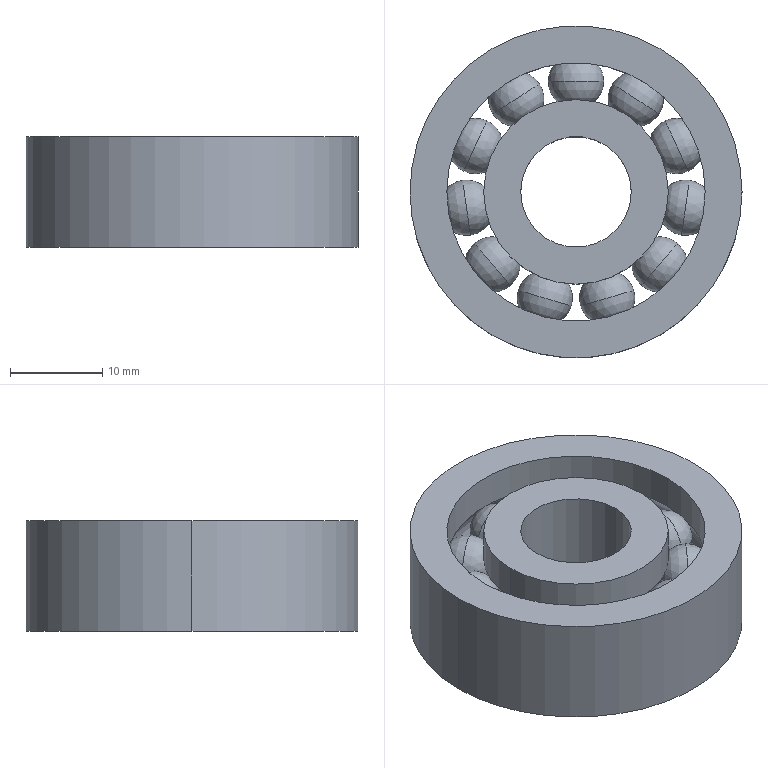Part | NX | features BREP 13 | 13 solids | 66 faces | box 36 x 36 x 12 mm | volume 8015 mm3 | sphere 44 | cylinder 12 | torus 6 | plane 4 | commonest cylinder face diameters 20 x4 28 x4 12 x2 36 x2
STEP:
#1=CARTESIAN_POINT('',(-10.916,4.985,3.));
#2=VERTEX_POINT('',#1);
#3=CARTESIAN_POINT('',(-9.669,7.714,0.));
#4=VERTEX_POINT('',#3);
#5=CARTESIAN_POINT('',(-10.916,4.985,0.));
#6=DIRECTION('',(-0.9096,0.4154,0.));
#7=DIRECTION('',(-0.4154,-0.9096,0.));
#8=AXIS2_PLACEMENT_3D('',#5,#6,#7);
#9=CIRCLE('',#8,3.);
#10=EDGE_CURVE('',#2,#4,#9,.T.);
#11=ORIENTED_EDGE('',*,*,#10,.F.);
#12=CARTESIAN_POINT('',(-12.162,2.256,0.));
#13=VERTEX_POINT('',#12);
#14=CARTESIAN_POINT('',(-10.916,4.985,0.));
#15=DIRECTION('',(0.9096,-0.4154,0.));
#16=DIRECTION('',(0.4154,0.9096,0.));
#17=AXIS2_PLACEMENT_3D('',#14,#15,#16);
#18=CIRCLE('',#17,3.);
#19=EDGE_CURVE('',#2,#13,#18,.T.);
#20=ORIENTED_EDGE('',*,*,#19,.T.);
#21=CARTESIAN_POINT('',(-10.916,4.985,0.));
#22=DIRECTION('',(0.,0.,1.));
#23=DIRECTION('',(1.,0.,0.));
#24=AXIS2_PLACEMENT_3D('',#21,#22,#23);
#25=CIRCLE('',#24,3.);
#26=EDGE_CURVE('',#13,#4,#25,.T.);
#27=ORIENTED_EDGE('',*,*,#26,.T.);
#28=EDGE_LOOP('',(#11,#20,#27));
#29=FACE_BOUND('',#28,.T.);
#30=CARTESIAN_POINT('',(-10.916,4.985,0.));
#31=DIRECTION('',(0.9096,-0.4154,0.));
#32=DIRECTION('',(-0.4154,-0.9096,0.));
#33=AXIS2_PLACEMENT_3D('',#30,#31,#32);
#34=SPHERICAL_SURFACE('',#33,3.);
#35=ADVANCED_FACE('',(#29),#34,.T.);
#36=ORIENTED_EDGE('',*,*,#26,.F.);
#37=CARTESIAN_POINT('',(-10.916,4.985,-3.));
#38=VERTEX_POINT('',#37);
#39=CARTESIAN_POINT('',(-10.916,4.985,0.));
#40=DIRECTION('',(0.9096,-0.4154,0.));
#41=DIRECTION('',(0.4154,0.9096,0.));
#42=AXIS2_PLACEMENT_3D('',#39,#40,#41);
#43=CIRCLE('',#42,3.);
#44=EDGE_CURVE('',#13,#38,#43,.T.);
#45=ORIENTED_EDGE('',*,*,#44,.T.);
#46=CARTESIAN_POINT('',(-10.916,4.985,0.));
#47=DIRECTION('',(-0.9096,0.4154,0.));
#48=DIRECTION('',(-0.4154,-0.9096,0.));
#49=AXIS2_PLACEMENT_3D('',#46,#47,#48);
#50=CIRCLE('',#49,3.);
#51=EDGE_CURVE('',#4,#38,#50,.T.);
#52=ORIENTED_EDGE('',*,*,#51,.F.);
#53=EDGE_LOOP('',(#36,#45,#52));
#54=FACE_BOUND('',#53,.T.);
#55=CARTESIAN_POINT('',(-10.916,4.985,0.));
#56=DIRECTION('',(0.9096,-0.4154,0.));
#57=DIRECTION('',(-0.4154,-0.9096,0.));
#58=AXIS2_PLACEMENT_3D('',#55,#56,#57);
#59=SPHERICAL_SURFACE('',#58,3.);
#60=ADVANCED_FACE('',(#54),#59,.T.);
#61=ORIENTED_EDGE('',*,*,#44,.F.);
#62=CARTESIAN_POINT('',(-10.916,4.985,0.));
#63=DIRECTION('',(0.,0.,1.));
#64=DIRECTION('',(1.,0.,0.));
#65=AXIS2_PLACEMENT_3D('',#62,#63,#64);
#66=CIRCLE('',#65,3.);
#67=EDGE_CURVE('',#4,#13,#66,.T.);
#68=ORIENTED_EDGE('',*,*,#67,.F.);
#69=ORIENTED_EDGE('',*,*,#51,.T.);
#70=EDGE_LOOP('',(#61,#68,#69));
#71=FACE_BOUND('',#70,.T.);
#72=CARTESIAN_POINT('',(-10.916,4.985,0.));
#73=DIRECTION('',(0.9096,-0.4154,0.));
#74=DIRECTION('',(-0.4154,-0.9096,0.));
#75=AXIS2_PLACEMENT_3D('',#72,#73,#74);
#76=SPHERICAL_SURFACE('',#75,3.);
#77=ADVANCED_FACE('',(#71),#76,.T.);
#78=ORIENTED_EDGE('',*,*,#19,.F.);
#79=ORIENTED_EDGE('',*,*,#10,.T.);
#80=ORIENTED_EDGE('',*,*,#67,.T.);
#81=EDGE_LOOP('',(#78,#79,#80));
#82=FACE_BOUND('',#81,.T.);
#83=CARTESIAN_POINT('',(-10.916,4.985,0.));
#84=DIRECTION('',(0.9096,-0.4154,0.));
#85=DIRECTION('',(-0.4154,-0.9096,0.));
#86=AXIS2_PLACEMENT_3D('',#83,#84,#85);
#87=SPHERICAL_SURFACE('',#86,3.);
#88=ADVANCED_FACE('',(#82),#87,.T.);
#89=CLOSED_SHELL('',(#35,#60,#77,#88));
#90=MANIFOLD_SOLID_BREP('',#89);
#91=CARTESIAN_POINT('',(10.916,4.985,3.));
#92=VERTEX_POINT('',#91);
#93=CARTESIAN_POINT('',(12.162,2.256,0.));
#94=VERTEX_POINT('',#93);
#95=CARTESIAN_POINT('',(10.916,4.985,0.));
#96=DIRECTION('',(0.9096,0.4154,0.));
#97=DIRECTION('',(-0.4154,0.9096,0.));
#98=AXIS2_PLACEMENT_3D('',#95,#96,#97);
#99=CIRCLE('',#98,3.);
#100=EDGE_CURVE('',#92,#94,#99,.T.);
#101=ORIENTED_EDGE('',*,*,#100,.F.);
#102=CARTESIAN_POINT('',(9.669,7.714,0.));
#103=VERTEX_POINT('',#102);
#104=CARTESIAN_POINT('',(10.916,4.985,0.));
#105=DIRECTION('',(-0.9096,-0.4154,0.));
#106=DIRECTION('',(0.4154,-0.9096,0.));
#107=AXIS2_PLACEMENT_3D('',#104,#105,#106);
#108=CIRCLE('',#107,3.);
#109=EDGE_CURVE('',#92,#103,#108,.T.);
#110=ORIENTED_EDGE('',*,*,#109,.T.);
#111=CARTESIAN_POINT('',(10.916,4.985,0.));
#112=DIRECTION('',(0.,0.,1.));
#113=DIRECTION('',(1.,0.,0.));
#114=AXIS2_PLACEMENT_3D('',#111,#112,#113);
#115=CIRCLE('',#114,3.);
#116=EDGE_CURVE('',#103,#94,#115,.T.);
#117=ORIENTED_EDGE('',*,*,#116,.T.);
#118=EDGE_LOOP('',(#101,#110,#117));
#119=FACE_BOUND('',#118,.T.);
#120=CARTESIAN_POINT('',(10.916,4.985,0.));
#121=DIRECTION('',(-0.9096,-0.4154,0.));
#122=DIRECTION('',(-0.4154,0.9096,0.));
#123=AXIS2_PLACEMENT_3D('',#120,#121,#122);
#124=SPHERICAL_SURFACE('',#123,3.);
#125=ADVANCED_FACE('',(#119),#124,.T.);
#126=ORIENTED_EDGE('',*,*,#116,.F.);
#127=CARTESIAN_POINT('',(10.916,4.985,-3.));
#128=VERTEX_POINT('',#127);
#129=CARTESIAN_POINT('',(10.916,4.985,0.));
#130=DIRECTION('',(-0.9096,-0.4154,0.));
#131=DIRECTION('',(0.4154,-0.9096,0.));
#132=AXIS2_PLACEMENT_3D('',#129,#130,#131);
#133=CIRCLE('',#132,3.);
#134=EDGE_CURVE('',#103,#128,#133,.T.);
#135=ORIENTED_EDGE('',*,*,#134,.T.);
#136=CARTESIAN_POINT('',(10.916,4.985,0.));
#137=DIRECTION('',(0.9096,0.4154,0.));
#138=DIRECTION('',(-0.4154,0.9096,0.));
#139=AXIS2_PLACEMENT_3D('',#136,#137,#138);
#140=CIRCLE('',#139,3.);
#141=EDGE_CURVE('',#94,#128,#140,.T.);
#142=ORIENTED_EDGE('',*,*,#141,.F.);
#143=EDGE_LOOP('',(#126,#135,#142));
#144=FACE_BOUND('',#143,.T.);
#145=CARTESIAN_POINT('',(10.916,4.985,0.));
#146=DIRECTION('',(-0.9096,-0.4154,0.));
#147=DIRECTION('',(-0.4154,0.9096,0.));
#148=AXIS2_PLACEMENT_3D('',#145,#146,#147);
#149=SPHERICAL_SURFACE('',#148,3.);
#150=ADVANCED_FACE('',(#144),#149,.T.);
#151=ORIENTED_EDGE('',*,*,#134,.F.);
#152=CARTESIAN_POINT('',(10.916,4.985,0.));
#153=DIRECTION('',(0.,0.,1.));
#154=DIRECTION('',(1.,0.,0.));
#155=AXIS2_PLACEMENT_3D('',#152,#153,#154);
#156=CIRCLE('',#155,3.);
#157=EDGE_CURVE('',#94,#103,#156,.T.);
#158=ORIENTED_EDGE('',*,*,#157,.F.);
#159=ORIENTED_EDGE('',*,*,#141,.T.);
#160=EDGE_LOOP('',(#151,#158,#159));
#161=FACE_BOUND('',#160,.T.);
#162=CARTESIAN_POINT('',(10.916,4.985,0.));
#163=DIRECTION('',(-0.9096,-0.4154,0.));
#164=DIRECTION('',(-0.4154,0.9096,0.));
#165=AXIS2_PLACEMENT_3D('',#162,#163,#164);
#166=SPHERICAL_SURFACE('',#165,3.);
#167=ADVANCED_FACE('',(#161),#166,.T.);
#168=ORIENTED_EDGE('',*,*,#109,.F.);
#169=ORIENTED_EDGE('',*,*,#100,.T.);
#170=ORIENTED_EDGE('',*,*,#157,.T.);
#171=EDGE_LOOP('',(#168,#169,#170));
#172=FACE_BOUND('',#171,.T.);
#173=CARTESIAN_POINT('',(10.916,4.985,0.));
#174=DIRECTION('',(-0.9096,-0.4154,0.));
#175=DIRECTION('',(-0.4154,0.9096,0.));
#176=AXIS2_PLACEMENT_3D('',#173,#174,#175);
#177=SPHERICAL_SURFACE('',#176,3.);
#178=ADVANCED_FACE('',(#172),#177,.T.);
#179=CLOSED_SHELL('',(#125,#150,#167,#178));
#180=MANIFOLD_SOLID_BREP('',#179);
#181=CARTESIAN_POINT('',(0.,12.,3.));
#182=VERTEX_POINT('',#181);
#183=CARTESIAN_POINT('',(3.,12.,0.));
#184=VERTEX_POINT('',#183);
#185=CARTESIAN_POINT('',(0.,12.,0.));
#186=DIRECTION('',(0.,1.,0.));
#187=DIRECTION('',(0.,0.,1.));
#188=AXIS2_PLACEMENT_3D('',#185,#186,#187);
#189=CIRCLE('',#188,3.);
#190=EDGE_CURVE('',#182,#184,#189,.T.);
#191=ORIENTED_EDGE('',*,*,#190,.F.);
#192=CARTESIAN_POINT('',(-3.,12.,0.));
#193=VERTEX_POINT('',#192);
#194=CARTESIAN_POINT('',(0.,12.,0.));
#195=DIRECTION('',(0.,-1.,0.));
#196=DIRECTION('',(1.,0.,0.));
#197=AXIS2_PLACEMENT_3D('',#194,#195,#196);
#198=CIRCLE('',#197,3.);
#199=EDGE_CURVE('',#182,#193,#198,.T.);
#200=ORIENTED_EDGE('',*,*,#199,.T.);
#201=CARTESIAN_POINT('',(0.,12.,0.));
#202=DIRECTION('',(0.,0.,1.));
#203=DIRECTION('',(1.,0.,0.));
#204=AXIS2_PLACEMENT_3D('',#201,#202,#203);
#205=CIRCLE('',#204,3.);
#206=EDGE_CURVE('',#193,#184,#205,.T.);
#207=ORIENTED_EDGE('',*,*,#206,.T.);
#208=EDGE_LOOP('',(#191,#200,#207));
#209=FACE_BOUND('',#208,.T.);
#210=CARTESIAN_POINT('',(0.,12.,0.));
#211=DIRECTION('',(0.,-1.,0.));
#212=DIRECTION('',(-1.,0.,0.));
#213=AXIS2_PLACEMENT_3D('',#210,#211,#212);
#214=SPHERICAL_SURFACE('',#213,3.);
#215=ADVANCED_FACE('',(#209),#214,.T.);
#216=ORIENTED_EDGE('',*,*,#206,.F.);
#217=CARTESIAN_POINT('',(0.,12.,-3.));
#218=VERTEX_POINT('',#217);
#219=CARTESIAN_POINT('',(0.,12.,0.));
#220=DIRECTION('',(0.,-1.,0.));
#221=DIRECTION('',(1.,0.,0.));
#222=AXIS2_PLACEMENT_3D('',#219,#220,#221);
#223=CIRCLE('',#222,3.);
#224=EDGE_CURVE('',#193,#218,#223,.T.);
#225=ORIENTED_EDGE('',*,*,#224,.T.);
#226=CARTESIAN_POINT('',(0.,12.,0.));
#227=DIRECTION('',(0.,1.,0.));
#228=DIRECTION('',(0.,0.,1.));
#229=AXIS2_PLACEMENT_3D('',#226,#227,#228);
#230=CIRCLE('',#229,3.);
#231=EDGE_CURVE('',#184,#218,#230,.T.);
#232=ORIENTED_EDGE('',*,*,#231,.F.);
#233=EDGE_LOOP('',(#216,#225,#232));
#234=FACE_BOUND('',#233,.T.);
#235=CARTESIAN_POINT('',(0.,12.,0.));
#236=DIRECTION('',(0.,-1.,0.));
#237=DIRECTION('',(-1.,0.,0.));
#238=AXIS2_PLACEMENT_3D('',#235,#236,#237);
#239=SPHERICAL_SURFACE('',#238,3.);
#240=ADVANCED_FACE('',(#234),#239,.T.);
#241=ORIENTED_EDGE('',*,*,#224,.F.);
#242=CARTESIAN_POINT('',(0.,12.,0.));
#243=DIRECTION('',(0.,0.,1.));
#244=DIRECTION('',(1.,0.,0.));
#245=AXIS2_PLACEMENT_3D('',#242,#243,#244);
#246=CIRCLE('',#245,3.);
#247=EDGE_CURVE('',#184,#193,#246,.T.);
#248=ORIENTED_EDGE('',*,*,#247,.F.);
#249=ORIENTED_EDGE('',*,*,#231,.T.);
#250=EDGE_LOOP('',(#241,#248,#249));
#251=FACE_BOUND('',#250,.T.);
#252=CARTESIAN_POINT('',(0.,12.,0.));
#253=DIRECTION('',(0.,-1.,0.));
#254=DIRECTION('',(-1.,0.,0.));
#255=AXIS2_PLACEMENT_3D('',#252,#253,#254);
#256=SPHERICAL_SURFACE('',#255,3.);
#257=ADVANCED_FACE('',(#251),#256,.T.);
#258=ORIENTED_EDGE('',*,*,#199,.F.);
#259=ORIENTED_EDGE('',*,*,#190,.T.);
#260=ORIENTED_EDGE('',*,*,#247,.T.);
#261=EDGE_LOOP('',(#258,#259,#260));
#262=FACE_BOUND('',#261,.T.);
#263=CARTESIAN_POINT('',(0.,12.,0.));
#264=DIRECTION('',(0.,-1.,0.));
#265=DIRECTION('',(-1.,0.,0.));
#266=AXIS2_PLACEMENT_3D('',#263,#264,#265);
#267=SPHERICAL_SURFACE('',#266,3.);
#268=ADVANCED_FACE('',(#262),#267,.T.);
#269=CLOSED_SHELL('',(#215,#240,#257,#268));
#270=MANIFOLD_SOLID_BREP('',#269);
#271=CARTESIAN_POINT('',(7.104,-10.126,0.));
#272=VERTEX_POINT('',#271);
#273=CARTESIAN_POINT('',(9.069,-7.858,3.));
#274=VERTEX_POINT('',#273);
#275=CARTESIAN_POINT('',(9.069,-7.858,0.));
#276=DIRECTION('',(0.7557,-0.6549,0.));
#277=DIRECTION('',(0.6549,0.7557,0.));
#278=AXIS2_PLACEMENT_3D('',#275,#276,#277);
#279=CIRCLE('',#278,3.);
#280=EDGE_CURVE('',#272,#274,#279,.F.);
#281=ORIENTED_EDGE('',*,*,#280,.T.);
#282=CARTESIAN_POINT('',(11.034,-5.591,0.));
#283=VERTEX_POINT('',#282);
#284=CARTESIAN_POINT('',(9.069,-7.858,0.));
#285=DIRECTION('',(-0.7557,0.6549,0.));
#286=DIRECTION('',(-0.6549,-0.7557,0.));
#287=AXIS2_PLACEMENT_3D('',#284,#285,#286);
#288=CIRCLE('',#287,3.);
#289=EDGE_CURVE('',#283,#274,#288,.F.);
#290=ORIENTED_EDGE('',*,*,#289,.F.);
#291=CARTESIAN_POINT('',(9.069,-7.858,0.));
#292=DIRECTION('',(0.,0.,1.));
#293=DIRECTION('',(1.,0.,0.));
#294=AXIS2_PLACEMENT_3D('',#291,#292,#293);
#295=CIRCLE('',#294,3.);
#296=EDGE_CURVE('',#283,#272,#295,.T.);
#297=ORIENTED_EDGE('',*,*,#296,.T.);
#298=EDGE_LOOP('',(#281,#290,#297));
#299=FACE_BOUND('',#298,.T.);
#300=CARTESIAN_POINT('',(9.069,-7.858,0.));
#301=DIRECTION('',(-0.7557,0.6549,0.));
#302=DIRECTION('',(0.6549,0.7557,0.));
#303=AXIS2_PLACEMENT_3D('',#300,#301,#302);
#304=SPHERICAL_SURFACE('',#303,3.);
#305=ADVANCED_FACE('',(#299),#304,.T.);
#306=ORIENTED_EDGE('',*,*,#296,.F.);
#307=CARTESIAN_POINT('',(9.069,-7.858,-3.));
#308=VERTEX_POINT('',#307);
#309=CARTESIAN_POINT('',(9.069,-7.858,0.));
#310=DIRECTION('',(-0.7557,0.6549,0.));
#311=DIRECTION('',(-0.6549,-0.7557,0.));
#312=AXIS2_PLACEMENT_3D('',#309,#310,#311);
#313=CIRCLE('',#312,3.);
#314=EDGE_CURVE('',#308,#283,#313,.F.);
#315=ORIENTED_EDGE('',*,*,#314,.F.);
#316=CARTESIAN_POINT('',(9.069,-7.858,0.));
#317=DIRECTION('',(0.7557,-0.6549,0.));
#318=DIRECTION('',(0.6549,0.7557,0.));
#319=AXIS2_PLACEMENT_3D('',#316,#317,#318);
#320=CIRCLE('',#319,3.);
#321=EDGE_CURVE('',#308,#272,#320,.F.);
#322=ORIENTED_EDGE('',*,*,#321,.T.);
#323=EDGE_LOOP('',(#306,#315,#322));
#324=FACE_BOUND('',#323,.T.);
#325=CARTESIAN_POINT('',(9.069,-7.858,0.));
#326=DIRECTION('',(-0.7557,0.6549,0.));
#327=DIRECTION('',(0.6549,0.7557,0.));
#328=AXIS2_PLACEMENT_3D('',#325,#326,#327);
#329=SPHERICAL_SURFACE('',#328,3.);
#330=ADVANCED_FACE('',(#324),#329,.T.);
#331=ORIENTED_EDGE('',*,*,#314,.T.);
#332=CARTESIAN_POINT('',(9.069,-7.858,0.));
#333=DIRECTION('',(0.,0.,1.));
#334=DIRECTION('',(1.,0.,0.));
#335=AXIS2_PLACEMENT_3D('',#332,#333,#334);
#336=CIRCLE('',#335,3.);
#337=EDGE_CURVE('',#272,#283,#336,.T.);
#338=ORIENTED_EDGE('',*,*,#337,.F.);
#339=ORIENTED_EDGE('',*,*,#321,.F.);
#340=EDGE_LOOP('',(#331,#338,#339));
#341=FACE_BOUND('',#340,.T.);
#342=CARTESIAN_POINT('',(9.069,-7.858,0.));
#343=DIRECTION('',(-0.7557,0.6549,0.));
#344=DIRECTION('',(0.6549,0.7557,0.));
#345=AXIS2_PLACEMENT_3D('',#342,#343,#344);
#346=SPHERICAL_SURFACE('',#345,3.);
#347=ADVANCED_FACE('',(#341),#346,.T.);
#348=ORIENTED_EDGE('',*,*,#289,.T.);
#349=ORIENTED_EDGE('',*,*,#280,.F.);
#350=ORIENTED_EDGE('',*,*,#337,.T.);
#351=EDGE_LOOP('',(#348,#349,#350));
#352=FACE_BOUND('',#351,.T.);
#353=CARTESIAN_POINT('',(9.069,-7.858,0.));
#354=DIRECTION('',(-0.7557,0.6549,0.));
#355=DIRECTION('',(0.6549,0.7557,0.));
#356=AXIS2_PLACEMENT_3D('',#353,#354,#355);
#357=SPHERICAL_SURFACE('',#356,3.);
#358=ADVANCED_FACE('',(#352),#357,.T.);
#359=CLOSED_SHELL('',(#305,#330,#347,#358));
#360=MANIFOLD_SOLID_BREP('',#359);
#361=CARTESIAN_POINT('',(-14.,0.,-2.236));
#362=VERTEX_POINT('',#361);
#363=CARTESIAN_POINT('',(14.,0.,-2.236));
#364=VERTEX_POINT('',#363);
#365=CARTESIAN_POINT('',(0.,0.,-2.236));
#366=DIRECTION('',(0.,0.,1.));
#367=DIRECTION('',(1.,0.,0.));
#368=AXIS2_PLACEMENT_3D('',#365,#366,#367);
#369=CIRCLE('',#368,14.);
#370=EDGE_CURVE('',#362,#364,#369,.T.);
#371=ORIENTED_EDGE('',*,*,#370,.F.);
#372=CARTESIAN_POINT('',(-14.,0.,2.236));
#373=VERTEX_POINT('',#372);
#374=CARTESIAN_POINT('',(-12.,0.,0.));
#375=DIRECTION('',(0.,1.,0.));
#376=DIRECTION('',(-1.,0.,0.));
#377=AXIS2_PLACEMENT_3D('',#374,#375,#376);
#378=CIRCLE('',#377,3.);
#379=EDGE_CURVE('',#362,#373,#378,.T.);
#380=ORIENTED_EDGE('',*,*,#379,.T.);
#381=CARTESIAN_POINT('',(14.,0.,2.236));
#382=VERTEX_POINT('',#381);
#383=CARTESIAN_POINT('',(0.,0.,2.236));
#384=DIRECTION('',(0.,0.,1.));
#385=DIRECTION('',(1.,0.,0.));
#386=AXIS2_PLACEMENT_3D('',#383,#384,#385);
#387=CIRCLE('',#386,14.);
#388=EDGE_CURVE('',#373,#382,#387,.T.);
#389=ORIENTED_EDGE('',*,*,#388,.T.);
#390=CARTESIAN_POINT('',(12.,0.,0.));
#391=DIRECTION('',(0.,-1.,0.));
#392=DIRECTION('',(1.,0.,0.));
#393=AXIS2_PLACEMENT_3D('',#390,#391,#392);
#394=CIRCLE('',#393,3.);
#395=EDGE_CURVE('',#364,#382,#394,.T.);
#396=ORIENTED_EDGE('',*,*,#395,.F.);
#397=EDGE_LOOP('',(#371,#380,#389,#396));
#398=FACE_BOUND('',#397,.T.);
#399=CARTESIAN_POINT('',(0.,0.,0.));
#400=DIRECTION('',(0.,0.,1.));
#401=DIRECTION('',(-1.,0.,0.));
#402=AXIS2_PLACEMENT_3D('',#399,#400,#401);
#403=TOROIDAL_SURFACE('',#402,12.,3.);
#404=ADVANCED_FACE('',(#398),#403,.F.);
#405=CARTESIAN_POINT('',(18.,0.,6.));
#406=VERTEX_POINT('',#405);
#407=CARTESIAN_POINT('',(-18.,0.,6.));
#408=VERTEX_POINT('',#407);
#409=CARTESIAN_POINT('',(0.,0.,6.));
#410=DIRECTION('',(0.,0.,1.));
#411=DIRECTION('',(1.,0.,0.));
#412=AXIS2_PLACEMENT_3D('',#409,#410,#411);
#413=CIRCLE('',#412,18.);
#414=EDGE_CURVE('',#406,#408,#413,.T.);
#415=ORIENTED_EDGE('',*,*,#414,.F.);
#416=CARTESIAN_POINT('',(18.,0.,-6.));
#417=VERTEX_POINT('',#416);
#418=CARTESIAN_POINT('',(18.,0.,6.));
#419=DIRECTION('',(0.,0.,-1.));
#420=VECTOR('',#419,1000.);
#421=LINE('',#418,#420);
#422=EDGE_CURVE('',#417,#406,#421,.F.);
#423=ORIENTED_EDGE('',*,*,#422,.F.);
#424=CARTESIAN_POINT('',(-18.,0.,-6.));
#425=VERTEX_POINT('',#424);
#426=CARTESIAN_POINT('',(0.,0.,-6.));
#427=DIRECTION('',(0.,0.,1.));
#428=DIRECTION('',(1.,0.,0.));
#429=AXIS2_PLACEMENT_3D('',#426,#427,#428);
#430=CIRCLE('',#429,18.);
#431=EDGE_CURVE('',#417,#425,#430,.T.);
#432=ORIENTED_EDGE('',*,*,#431,.T.);
#433=CARTESIAN_POINT('',(-18.,0.,6.));
#434=DIRECTION('',(0.,0.,-1.));
#435=VECTOR('',#434,1000.);
#436=LINE('',#433,#435);
#437=EDGE_CURVE('',#425,#408,#436,.F.);
#438=ORIENTED_EDGE('',*,*,#437,.T.);
#439=EDGE_LOOP('',(#415,#423,#432,#438));
#440=FACE_BOUND('',#439,.T.);
#441=CARTESIAN_POINT('',(0.,0.,6.));
#442=DIRECTION('',(0.,0.,-1.));
#443=DIRECTION('',(1.,0.,0.));
#444=AXIS2_PLACEMENT_3D('',#441,#442,#443);
#445=CYLINDRICAL_SURFACE('',#444,18.);
#446=ADVANCED_FACE('',(#440),#445,.T.);
#447=ORIENTED_EDGE('',*,*,#370,.T.);
#448=CARTESIAN_POINT('',(14.,0.,-6.));
#449=VERTEX_POINT('',#448);
#450=CARTESIAN_POINT('',(14.,0.,6.));
#451=DIRECTION('',(0.,0.,-1.));
#452=VECTOR('',#451,1000.);
#453=LINE('',#450,#452);
#454=EDGE_CURVE('',#449,#364,#453,.F.);
#455=ORIENTED_EDGE('',*,*,#454,.F.);
#456=CARTESIAN_POINT('',(-14.,0.,-6.));
#457=VERTEX_POINT('',#456);
#458=CARTESIAN_POINT('',(0.,0.,-6.));
#459=DIRECTION('',(0.,0.,1.));
#460=DIRECTION('',(1.,0.,0.));
#461=AXIS2_PLACEMENT_3D('',#458,#459,#460);
#462=CIRCLE('',#461,14.);
#463=EDGE_CURVE('',#457,#449,#462,.T.);
#464=ORIENTED_EDGE('',*,*,#463,.F.);
#465=CARTESIAN_POINT('',(-14.,0.,6.));
#466=DIRECTION('',(0.,0.,-1.));
#467=VECTOR('',#466,1000.);
#468=LINE('',#465,#467);
#469=EDGE_CURVE('',#457,#362,#468,.F.);
#470=ORIENTED_EDGE('',*,*,#469,.T.);
#471=EDGE_LOOP('',(#447,#455,#464,#470));
#472=FACE_BOUND('',#471,.T.);
#473=CARTESIAN_POINT('',(0.,0.,6.));
#474=DIRECTION('',(0.,0.,-1.));
#475=DIRECTION('',(1.,0.,0.));
#476=AXIS2_PLACEMENT_3D('',#473,#474,#475);
#477=CYLINDRICAL_SURFACE('',#476,14.);
#478=ADVANCED_FACE('',(#472),#477,.F.);
#479=CARTESIAN_POINT('',(-14.,0.,6.));
#480=VERTEX_POINT('',#479);
#481=CARTESIAN_POINT('',(14.,0.,6.));
#482=VERTEX_POINT('',#481);
#483=CARTESIAN_POINT('',(0.,0.,6.));
#484=DIRECTION('',(0.,0.,1.));
#485=DIRECTION('',(1.,0.,0.));
#486=AXIS2_PLACEMENT_3D('',#483,#484,#485);
#487=CIRCLE('',#486,14.);
#488=EDGE_CURVE('',#480,#482,#487,.T.);
#489=ORIENTED_EDGE('',*,*,#488,.T.);
#490=CARTESIAN_POINT('',(14.,0.,6.));
#491=DIRECTION('',(0.,0.,-1.));
#492=VECTOR('',#491,1000.);
#493=LINE('',#490,#492);
#494=EDGE_CURVE('',#382,#482,#493,.F.);
#495=ORIENTED_EDGE('',*,*,#494,.F.);
#496=ORIENTED_EDGE('',*,*,#388,.F.);
#497=CARTESIAN_POINT('',(-14.,0.,6.));
#498=DIRECTION('',(0.,0.,-1.));
#499=VECTOR('',#498,1000.);
#500=LINE('',#497,#499);
#501=EDGE_CURVE('',#373,#480,#500,.F.);
#502=ORIENTED_EDGE('',*,*,#501,.T.);
#503=EDGE_LOOP('',(#489,#495,#496,#502));
#504=FACE_BOUND('',#503,.T.);
#505=CARTESIAN_POINT('',(0.,0.,6.));
#506=DIRECTION('',(0.,0.,-1.));
#507=DIRECTION('',(1.,0.,0.));
#508=AXIS2_PLACEMENT_3D('',#505,#506,#507);
#509=CYLINDRICAL_SURFACE('',#508,14.);
#510=ADVANCED_FACE('',(#504),#509,.F.);
#511=ORIENTED_EDGE('',*,*,#494,.T.);
#512=CARTESIAN_POINT('',(0.,0.,6.));
#513=DIRECTION('',(0.,0.,1.));
#514=DIRECTION('',(1.,0.,0.));
#515=AXIS2_PLACEMENT_3D('',#512,#513,#514);
#516=CIRCLE('',#515,14.);
#517=EDGE_CURVE('',#482,#480,#516,.T.);
#518=ORIENTED_EDGE('',*,*,#517,.T.);
#519=ORIENTED_EDGE('',*,*,#501,.F.);
#520=CARTESIAN_POINT('',(0.,0.,2.236));
#521=DIRECTION('',(0.,0.,1.));
#522=DIRECTION('',(1.,0.,0.));
#523=AXIS2_PLACEMENT_3D('',#520,#521,#522);
#524=CIRCLE('',#523,14.);
#525=EDGE_CURVE('',#382,#373,#524,.T.);
#526=ORIENTED_EDGE('',*,*,#525,.F.);
#527=EDGE_LOOP('',(#511,#518,#519,#526));
#528=FACE_BOUND('',#527,.T.);
#529=CARTESIAN_POINT('',(0.,0.,6.));
#530=DIRECTION('',(0.,0.,-1.));
#531=DIRECTION('',(1.,0.,0.));
#532=AXIS2_PLACEMENT_3D('',#529,#530,#531);
#533=CYLINDRICAL_SURFACE('',#532,14.);
#534=ADVANCED_FACE('',(#528),#533,.F.);
#535=ORIENTED_EDGE('',*,*,#454,.T.);
#536=CARTESIAN_POINT('',(0.,0.,-2.236));
#537=DIRECTION('',(0.,0.,1.));
#538=DIRECTION('',(1.,0.,0.));
#539=AXIS2_PLACEMENT_3D('',#536,#537,#538);
#540=CIRCLE('',#539,14.);
#541=EDGE_CURVE('',#364,#362,#540,.T.);
#542=ORIENTED_EDGE('',*,*,#541,.T.);
#543=ORIENTED_EDGE('',*,*,#469,.F.);
#544=CARTESIAN_POINT('',(0.,0.,-6.));
#545=DIRECTION('',(0.,0.,1.));
#546=DIRECTION('',(1.,0.,0.));
#547=AXIS2_PLACEMENT_3D('',#544,#545,#546);
#548=CIRCLE('',#547,14.);
#549=EDGE_CURVE('',#449,#457,#548,.T.);
#550=ORIENTED_EDGE('',*,*,#549,.F.);
#551=EDGE_LOOP('',(#535,#542,#543,#550));
#552=FACE_BOUND('',#551,.T.);
#553=CARTESIAN_POINT('',(0.,0.,6.));
#554=DIRECTION('',(0.,0.,-1.));
#555=DIRECTION('',(1.,0.,0.));
#556=AXIS2_PLACEMENT_3D('',#553,#554,#555);
#557=CYLINDRICAL_SURFACE('',#556,14.);
#558=ADVANCED_FACE('',(#552),#557,.F.);
#559=ORIENTED_EDGE('',*,*,#422,.T.);
#560=CARTESIAN_POINT('',(0.,0.,6.));
#561=DIRECTION('',(0.,0.,1.));
#562=DIRECTION('',(1.,0.,0.));
#563=AXIS2_PLACEMENT_3D('',#560,#561,#562);
#564=CIRCLE('',#563,18.);
#565=EDGE_CURVE('',#408,#406,#564,.T.);
#566=ORIENTED_EDGE('',*,*,#565,.F.);
#567=ORIENTED_EDGE('',*,*,#437,.F.);
#568=CARTESIAN_POINT('',(0.,0.,-6.));
#569=DIRECTION('',(0.,0.,1.));
#570=DIRECTION('',(1.,0.,0.));
#571=AXIS2_PLACEMENT_3D('',#568,#569,#570);
#572=CIRCLE('',#571,18.);
#573=EDGE_CURVE('',#425,#417,#572,.T.);
#574=ORIENTED_EDGE('',*,*,#573,.T.);
#575=EDGE_LOOP('',(#559,#566,#567,#574));
#576=FACE_BOUND('',#575,.T.);
#577=CARTESIAN_POINT('',(0.,0.,6.));
#578=DIRECTION('',(0.,0.,-1.));
#579=DIRECTION('',(1.,0.,0.));
#580=AXIS2_PLACEMENT_3D('',#577,#578,#579);
#581=CYLINDRICAL_SURFACE('',#580,18.);
#582=ADVANCED_FACE('',(#576),#581,.T.);
#583=ORIENTED_EDGE('',*,*,#565,.T.);
#584=ORIENTED_EDGE('',*,*,#414,.T.);
#585=EDGE_LOOP('',(#583,#584));
#586=FACE_BOUND('',#585,.T.);
#587=ORIENTED_EDGE('',*,*,#488,.F.);
#588=ORIENTED_EDGE('',*,*,#517,.F.);
#589=EDGE_LOOP('',(#587,#588));
#590=FACE_BOUND('',#589,.T.);
#591=CARTESIAN_POINT('',(0.,0.,6.));
#592=DIRECTION('',(0.,0.,1.));
#593=DIRECTION('',(-1.,0.,0.));
#594=AXIS2_PLACEMENT_3D('',#591,#592,#593);
#595=PLANE('',#594);
#596=ADVANCED_FACE('',(#586,#590),#595,.T.);
#597=ORIENTED_EDGE('',*,*,#573,.F.);
#598=ORIENTED_EDGE('',*,*,#431,.F.);
#599=EDGE_LOOP('',(#597,#598));
#600=FACE_BOUND('',#599,.T.);
#601=ORIENTED_EDGE('',*,*,#463,.T.);
#602=ORIENTED_EDGE('',*,*,#549,.T.);
#603=EDGE_LOOP('',(#601,#602));
#604=FACE_BOUND('',#603,.T.);
#605=CARTESIAN_POINT('',(0.,0.,-6.));
#606=DIRECTION('',(0.,0.,1.));
#607=DIRECTION('',(-1.,0.,0.));
#608=AXIS2_PLACEMENT_3D('',#605,#606,#607);
#609=PLANE('',#608);
#610=ADVANCED_FACE('',(#600,#604),#609,.F.);
#611=ORIENTED_EDGE('',*,*,#379,.F.);
#612=ORIENTED_EDGE('',*,*,#541,.F.);
#613=ORIENTED_EDGE('',*,*,#395,.T.);
#614=ORIENTED_EDGE('',*,*,#525,.T.);
#615=EDGE_LOOP('',(#611,#612,#613,#614));
#616=FACE_BOUND('',#615,.T.);
#617=CARTESIAN_POINT('',(0.,0.,0.));
#618=DIRECTION('',(0.,0.,1.));
#619=DIRECTION('',(-1.,0.,0.));
#620=AXIS2_PLACEMENT_3D('',#617,#618,#619);
#621=TOROIDAL_SURFACE('',#620,12.,3.);
#622=ADVANCED_FACE('',(#616),#621,.F.);
#623=CLOSED_SHELL('',(#404,#446,#478,#510,#534,#558,#582,#596,#610,#622));
#624=MANIFOLD_SOLID_BREP('',#623);
#625=CARTESIAN_POINT('',(-6.259,-10.669,0.));
#626=VERTEX_POINT('',#625);
#627=CARTESIAN_POINT('',(-3.381,-11.514,3.));
#628=VERTEX_POINT('',#627);
#629=CARTESIAN_POINT('',(-3.381,-11.514,0.));
#630=DIRECTION('',(-0.2817,-0.9595,0.));
#631=DIRECTION('',(0.9595,-0.2817,0.));
#632=AXIS2_PLACEMENT_3D('',#629,#630,#631);
#633=CIRCLE('',#632,3.);
#634=EDGE_CURVE('',#626,#628,#633,.F.);
#635=ORIENTED_EDGE('',*,*,#634,.T.);
#636=CARTESIAN_POINT('',(-0.5023,-12.359,0.));
#637=VERTEX_POINT('',#636);
#638=CARTESIAN_POINT('',(-3.381,-11.514,0.));
#639=DIRECTION('',(0.2817,0.9595,0.));
#640=DIRECTION('',(-0.9595,0.2817,0.));
#641=AXIS2_PLACEMENT_3D('',#638,#639,#640);
#642=CIRCLE('',#641,3.);
#643=EDGE_CURVE('',#637,#628,#642,.F.);
#644=ORIENTED_EDGE('',*,*,#643,.F.);
#645=CARTESIAN_POINT('',(-3.381,-11.514,0.));
#646=DIRECTION('',(0.,0.,1.));
#647=DIRECTION('',(1.,0.,0.));
#648=AXIS2_PLACEMENT_3D('',#645,#646,#647);
#649=CIRCLE('',#648,3.);
#650=EDGE_CURVE('',#637,#626,#649,.T.);
#651=ORIENTED_EDGE('',*,*,#650,.T.);
#652=EDGE_LOOP('',(#635,#644,#651));
#653=FACE_BOUND('',#652,.T.);
#654=CARTESIAN_POINT('',(-3.381,-11.514,0.));
#655=DIRECTION('',(0.2817,0.9595,0.));
#656=DIRECTION('',(0.9595,-0.2817,0.));
#657=AXIS2_PLACEMENT_3D('',#654,#655,#656);
#658=SPHERICAL_SURFACE('',#657,3.);
#659=ADVANCED_FACE('',(#653),#658,.T.);
#660=ORIENTED_EDGE('',*,*,#650,.F.);
#661=CARTESIAN_POINT('',(-3.381,-11.514,-3.));
#662=VERTEX_POINT('',#661);
#663=CARTESIAN_POINT('',(-3.381,-11.514,0.));
#664=DIRECTION('',(0.2817,0.9595,0.));
#665=DIRECTION('',(-0.9595,0.2817,0.));
#666=AXIS2_PLACEMENT_3D('',#663,#664,#665);
#667=CIRCLE('',#666,3.);
#668=EDGE_CURVE('',#662,#637,#667,.F.);
#669=ORIENTED_EDGE('',*,*,#668,.F.);
#670=CARTESIAN_POINT('',(-3.381,-11.514,0.));
#671=DIRECTION('',(-0.2817,-0.9595,0.));
#672=DIRECTION('',(0.9595,-0.2817,0.));
#673=AXIS2_PLACEMENT_3D('',#670,#671,#672);
#674=CIRCLE('',#673,3.);
#675=EDGE_CURVE('',#662,#626,#674,.F.);
#676=ORIENTED_EDGE('',*,*,#675,.T.);
#677=EDGE_LOOP('',(#660,#669,#676));
#678=FACE_BOUND('',#677,.T.);
#679=CARTESIAN_POINT('',(-3.381,-11.514,0.));
#680=DIRECTION('',(0.2817,0.9595,0.));
#681=DIRECTION('',(0.9595,-0.2817,0.));
#682=AXIS2_PLACEMENT_3D('',#679,#680,#681);
#683=SPHERICAL_SURFACE('',#682,3.);
#684=ADVANCED_FACE('',(#678),#683,.T.);
#685=ORIENTED_EDGE('',*,*,#668,.T.);
#686=CARTESIAN_POINT('',(-3.381,-11.514,0.));
#687=DIRECTION('',(0.,0.,1.));
#688=DIRECTION('',(1.,0.,0.));
#689=AXIS2_PLACEMENT_3D('',#686,#687,#688);
#690=CIRCLE('',#689,3.);
#691=EDGE_CURVE('',#626,#637,#690,.T.);
#692=ORIENTED_EDGE('',*,*,#691,.F.);
#693=ORIENTED_EDGE('',*,*,#675,.F.);
#694=EDGE_LOOP('',(#685,#692,#693));
#695=FACE_BOUND('',#694,.T.);
#696=CARTESIAN_POINT('',(-3.381,-11.514,0.));
#697=DIRECTION('',(0.2817,0.9595,0.));
#698=DIRECTION('',(0.9595,-0.2817,0.));
#699=AXIS2_PLACEMENT_3D('',#696,#697,#698);
#700=SPHERICAL_SURFACE('',#699,3.);
#701=ADVANCED_FACE('',(#695),#700,.T.);
#702=ORIENTED_EDGE('',*,*,#643,.T.);
#703=ORIENTED_EDGE('',*,*,#634,.F.);
#704=ORIENTED_EDGE('',*,*,#691,.T.);
#705=EDGE_LOOP('',(#702,#703,#704));
#706=FACE_BOUND('',#705,.T.);
#707=CARTESIAN_POINT('',(-3.381,-11.514,0.));
#708=DIRECTION('',(0.2817,0.9595,0.));
#709=DIRECTION('',(0.9595,-0.2817,0.));
#710=AXIS2_PLACEMENT_3D('',#707,#708,#709);
#711=SPHERICAL_SURFACE('',#710,3.);
#712=ADVANCED_FACE('',(#706),#711,.T.);
#713=CLOSED_SHELL('',(#659,#684,#701,#712));
#714=MANIFOLD_SOLID_BREP('',#713);
#715=CARTESIAN_POINT('',(-12.305,1.262,0.));
#716=VERTEX_POINT('',#715);
#717=CARTESIAN_POINT('',(-11.878,-1.708,3.));
#718=VERTEX_POINT('',#717);
#719=CARTESIAN_POINT('',(-11.878,-1.708,0.));
#720=DIRECTION('',(-0.9898,-0.1423,0.));
#721=DIRECTION('',(0.1423,-0.9898,0.));
#722=AXIS2_PLACEMENT_3D('',#719,#720,#721);
#723=CIRCLE('',#722,3.);
#724=EDGE_CURVE('',#716,#718,#723,.F.);
#725=ORIENTED_EDGE('',*,*,#724,.T.);
#726=CARTESIAN_POINT('',(-11.451,-4.677,0.));
#727=VERTEX_POINT('',#726);
#728=CARTESIAN_POINT('',(-11.878,-1.708,0.));
#729=DIRECTION('',(0.9898,0.1423,0.));
#730=DIRECTION('',(-0.1423,0.9898,0.));
#731=AXIS2_PLACEMENT_3D('',#728,#729,#730);
#732=CIRCLE('',#731,3.);
#733=EDGE_CURVE('',#727,#718,#732,.F.);
#734=ORIENTED_EDGE('',*,*,#733,.F.);
#735=CARTESIAN_POINT('',(-11.878,-1.708,0.));
#736=DIRECTION('',(0.,0.,1.));
#737=DIRECTION('',(1.,0.,0.));
#738=AXIS2_PLACEMENT_3D('',#735,#736,#737);
#739=CIRCLE('',#738,3.);
#740=EDGE_CURVE('',#727,#716,#739,.T.);
#741=ORIENTED_EDGE('',*,*,#740,.T.);
#742=EDGE_LOOP('',(#725,#734,#741));
#743=FACE_BOUND('',#742,.T.);
#744=CARTESIAN_POINT('',(-11.878,-1.708,0.));
#745=DIRECTION('',(0.9898,0.1423,0.));
#746=DIRECTION('',(0.1423,-0.9898,0.));
#747=AXIS2_PLACEMENT_3D('',#744,#745,#746);
#748=SPHERICAL_SURFACE('',#747,3.);
#749=ADVANCED_FACE('',(#743),#748,.T.);
#750=ORIENTED_EDGE('',*,*,#740,.F.);
#751=CARTESIAN_POINT('',(-11.878,-1.708,-3.));
#752=VERTEX_POINT('',#751);
#753=CARTESIAN_POINT('',(-11.878,-1.708,0.));
#754=DIRECTION('',(0.9898,0.1423,0.));
#755=DIRECTION('',(-0.1423,0.9898,0.));
#756=AXIS2_PLACEMENT_3D('',#753,#754,#755);
#757=CIRCLE('',#756,3.);
#758=EDGE_CURVE('',#752,#727,#757,.F.);
#759=ORIENTED_EDGE('',*,*,#758,.F.);
#760=CARTESIAN_POINT('',(-11.878,-1.708,0.));
#761=DIRECTION('',(-0.9898,-0.1423,0.));
#762=DIRECTION('',(0.1423,-0.9898,0.));
#763=AXIS2_PLACEMENT_3D('',#760,#761,#762);
#764=CIRCLE('',#763,3.);
#765=EDGE_CURVE('',#752,#716,#764,.F.);
#766=ORIENTED_EDGE('',*,*,#765,.T.);
#767=EDGE_LOOP('',(#750,#759,#766));
#768=FACE_BOUND('',#767,.T.);
#769=CARTESIAN_POINT('',(-11.878,-1.708,0.));
#770=DIRECTION('',(0.9898,0.1423,0.));
#771=DIRECTION('',(0.1423,-0.9898,0.));
#772=AXIS2_PLACEMENT_3D('',#769,#770,#771);
#773=SPHERICAL_SURFACE('',#772,3.);
#774=ADVANCED_FACE('',(#768),#773,.T.);
#775=ORIENTED_EDGE('',*,*,#758,.T.);
#776=CARTESIAN_POINT('',(-11.878,-1.708,0.));
#777=DIRECTION('',(0.,0.,1.));
#778=DIRECTION('',(1.,0.,0.));
#779=AXIS2_PLACEMENT_3D('',#776,#777,#778);
#780=CIRCLE('',#779,3.);
#781=EDGE_CURVE('',#716,#727,#780,.T.);
#782=ORIENTED_EDGE('',*,*,#781,.F.);
#783=ORIENTED_EDGE('',*,*,#765,.F.);
#784=EDGE_LOOP('',(#775,#782,#783));
#785=FACE_BOUND('',#784,.T.);
#786=CARTESIAN_POINT('',(-11.878,-1.708,0.));
#787=DIRECTION('',(0.9898,0.1423,0.));
#788=DIRECTION('',(0.1423,-0.9898,0.));
#789=AXIS2_PLACEMENT_3D('',#786,#787,#788);
#790=SPHERICAL_SURFACE('',#789,3.);
#791=ADVANCED_FACE('',(#785),#790,.T.);
#792=ORIENTED_EDGE('',*,*,#733,.T.);
#793=ORIENTED_EDGE('',*,*,#724,.F.);
#794=ORIENTED_EDGE('',*,*,#781,.T.);
#795=EDGE_LOOP('',(#792,#793,#794));
#796=FACE_BOUND('',#795,.T.);
#797=CARTESIAN_POINT('',(-11.878,-1.708,0.));
#798=DIRECTION('',(0.9898,0.1423,0.));
#799=DIRECTION('',(0.1423,-0.9898,0.));
#800=AXIS2_PLACEMENT_3D('',#797,#798,#799);
#801=SPHERICAL_SURFACE('',#800,3.);
#802=ADVANCED_FACE('',(#796),#801,.T.);
#803=CLOSED_SHELL('',(#749,#774,#791,#802));
#804=MANIFOLD_SOLID_BREP('',#803);
#805=CARTESIAN_POINT('',(6.488,10.095,3.));
#806=VERTEX_POINT('',#805);
#807=CARTESIAN_POINT('',(9.011,8.473,0.));
#808=VERTEX_POINT('',#807);
#809=CARTESIAN_POINT('',(6.488,10.095,0.));
#810=DIRECTION('',(0.5406,0.8413,0.));
#811=DIRECTION('',(-0.8413,0.5406,0.));
#812=AXIS2_PLACEMENT_3D('',#809,#810,#811);
#813=CIRCLE('',#812,3.);
#814=EDGE_CURVE('',#806,#808,#813,.T.);
#815=ORIENTED_EDGE('',*,*,#814,.F.);
#816=CARTESIAN_POINT('',(3.964,11.717,0.));
#817=VERTEX_POINT('',#816);
#818=CARTESIAN_POINT('',(6.488,10.095,0.));
#819=DIRECTION('',(-0.5406,-0.8413,0.));
#820=DIRECTION('',(0.8413,-0.5406,0.));
#821=AXIS2_PLACEMENT_3D('',#818,#819,#820);
#822=CIRCLE('',#821,3.);
#823=EDGE_CURVE('',#806,#817,#822,.T.);
#824=ORIENTED_EDGE('',*,*,#823,.T.);
#825=CARTESIAN_POINT('',(6.488,10.095,0.));
#826=DIRECTION('',(0.,0.,1.));
#827=DIRECTION('',(1.,0.,0.));
#828=AXIS2_PLACEMENT_3D('',#825,#826,#827);
#829=CIRCLE('',#828,3.);
#830=EDGE_CURVE('',#817,#808,#829,.T.);
#831=ORIENTED_EDGE('',*,*,#830,.T.);
#832=EDGE_LOOP('',(#815,#824,#831));
#833=FACE_BOUND('',#832,.T.);
#834=CARTESIAN_POINT('',(6.488,10.095,0.));
#835=DIRECTION('',(-0.5406,-0.8413,0.));
#836=DIRECTION('',(-0.8413,0.5406,0.));
#837=AXIS2_PLACEMENT_3D('',#834,#835,#836);
#838=SPHERICAL_SURFACE('',#837,3.);
#839=ADVANCED_FACE('',(#833),#838,.T.);
#840=ORIENTED_EDGE('',*,*,#830,.F.);
#841=CARTESIAN_POINT('',(6.488,10.095,-3.));
#842=VERTEX_POINT('',#841);
#843=CARTESIAN_POINT('',(6.488,10.095,0.));
#844=DIRECTION('',(-0.5406,-0.8413,0.));
#845=DIRECTION('',(0.8413,-0.5406,0.));
#846=AXIS2_PLACEMENT_3D('',#843,#844,#845);
#847=CIRCLE('',#846,3.);
#848=EDGE_CURVE('',#817,#842,#847,.T.);
#849=ORIENTED_EDGE('',*,*,#848,.T.);
#850=CARTESIAN_POINT('',(6.488,10.095,0.));
#851=DIRECTION('',(0.5406,0.8413,0.));
#852=DIRECTION('',(-0.8413,0.5406,0.));
#853=AXIS2_PLACEMENT_3D('',#850,#851,#852);
#854=CIRCLE('',#853,3.);
#855=EDGE_CURVE('',#808,#842,#854,.T.);
#856=ORIENTED_EDGE('',*,*,#855,.F.);
#857=EDGE_LOOP('',(#840,#849,#856));
#858=FACE_BOUND('',#857,.T.);
#859=CARTESIAN_POINT('',(6.488,10.095,0.));
#860=DIRECTION('',(-0.5406,-0.8413,0.));
#861=DIRECTION('',(-0.8413,0.5406,0.));
#862=AXIS2_PLACEMENT_3D('',#859,#860,#861);
#863=SPHERICAL_SURFACE('',#862,3.);
#864=ADVANCED_FACE('',(#858),#863,.T.);
#865=ORIENTED_EDGE('',*,*,#848,.F.);
#866=CARTESIAN_POINT('',(6.488,10.095,0.));
#867=DIRECTION('',(0.,0.,1.));
#868=DIRECTION('',(1.,0.,0.));
#869=AXIS2_PLACEMENT_3D('',#866,#867,#868);
#870=CIRCLE('',#869,3.);
#871=EDGE_CURVE('',#808,#817,#870,.T.);
#872=ORIENTED_EDGE('',*,*,#871,.F.);
#873=ORIENTED_EDGE('',*,*,#855,.T.);
#874=EDGE_LOOP('',(#865,#872,#873));
#875=FACE_BOUND('',#874,.T.);
#876=CARTESIAN_POINT('',(6.488,10.095,0.));
#877=DIRECTION('',(-0.5406,-0.8413,0.));
#878=DIRECTION('',(-0.8413,0.5406,0.));
#879=AXIS2_PLACEMENT_3D('',#876,#877,#878);
#880=SPHERICAL_SURFACE('',#879,3.);
#881=ADVANCED_FACE('',(#875),#880,.T.);
#882=ORIENTED_EDGE('',*,*,#823,.F.);
#883=ORIENTED_EDGE('',*,*,#814,.T.);
#884=ORIENTED_EDGE('',*,*,#871,.T.);
#885=EDGE_LOOP('',(#882,#883,#884));
#886=FACE_BOUND('',#885,.T.);
#887=CARTESIAN_POINT('',(6.488,10.095,0.));
#888=DIRECTION('',(-0.5406,-0.8413,0.));
#889=DIRECTION('',(-0.8413,0.5406,0.));
#890=AXIS2_PLACEMENT_3D('',#887,#888,#889);
#891=SPHERICAL_SURFACE('',#890,3.);
#892=ADVANCED_FACE('',(#886),#891,.T.);
#893=CLOSED_SHELL('',(#839,#864,#881,#892));
#894=MANIFOLD_SOLID_BREP('',#893);
#895=CARTESIAN_POINT('',(-6.488,10.095,3.));
#896=VERTEX_POINT('',#895);
#897=CARTESIAN_POINT('',(-3.964,11.717,0.));
#898=VERTEX_POINT('',#897);
#899=CARTESIAN_POINT('',(-6.488,10.095,0.));
#900=DIRECTION('',(-0.5406,0.8413,0.));
#901=DIRECTION('',(-0.8413,-0.5406,0.));
#902=AXIS2_PLACEMENT_3D('',#899,#900,#901);
#903=CIRCLE('',#902,3.);
#904=EDGE_CURVE('',#896,#898,#903,.T.);
#905=ORIENTED_EDGE('',*,*,#904,.F.);
#906=CARTESIAN_POINT('',(-9.011,8.473,0.));
#907=VERTEX_POINT('',#906);
#908=CARTESIAN_POINT('',(-6.488,10.095,0.));
#909=DIRECTION('',(0.5406,-0.8413,0.));
#910=DIRECTION('',(0.8413,0.5406,0.));
#911=AXIS2_PLACEMENT_3D('',#908,#909,#910);
#912=CIRCLE('',#911,3.);
#913=EDGE_CURVE('',#896,#907,#912,.T.);
#914=ORIENTED_EDGE('',*,*,#913,.T.);
#915=CARTESIAN_POINT('',(-6.488,10.095,0.));
#916=DIRECTION('',(0.,0.,1.));
#917=DIRECTION('',(1.,0.,0.));
#918=AXIS2_PLACEMENT_3D('',#915,#916,#917);
#919=CIRCLE('',#918,3.);
#920=EDGE_CURVE('',#907,#898,#919,.T.);
#921=ORIENTED_EDGE('',*,*,#920,.T.);
#922=EDGE_LOOP('',(#905,#914,#921));
#923=FACE_BOUND('',#922,.T.);
#924=CARTESIAN_POINT('',(-6.488,10.095,0.));
#925=DIRECTION('',(0.5406,-0.8413,0.));
#926=DIRECTION('',(-0.8413,-0.5406,0.));
#927=AXIS2_PLACEMENT_3D('',#924,#925,#926);
#928=SPHERICAL_SURFACE('',#927,3.);
#929=ADVANCED_FACE('',(#923),#928,.T.);
#930=ORIENTED_EDGE('',*,*,#920,.F.);
#931=CARTESIAN_POINT('',(-6.488,10.095,-3.));
#932=VERTEX_POINT('',#931);
#933=CARTESIAN_POINT('',(-6.488,10.095,0.));
#934=DIRECTION('',(0.5406,-0.8413,0.));
#935=DIRECTION('',(0.8413,0.5406,0.));
#936=AXIS2_PLACEMENT_3D('',#933,#934,#935);
#937=CIRCLE('',#936,3.);
#938=EDGE_CURVE('',#907,#932,#937,.T.);
#939=ORIENTED_EDGE('',*,*,#938,.T.);
#940=CARTESIAN_POINT('',(-6.488,10.095,0.));
#941=DIRECTION('',(-0.5406,0.8413,0.));
#942=DIRECTION('',(-0.8413,-0.5406,0.));
#943=AXIS2_PLACEMENT_3D('',#940,#941,#942);
#944=CIRCLE('',#943,3.);
#945=EDGE_CURVE('',#898,#932,#944,.T.);
#946=ORIENTED_EDGE('',*,*,#945,.F.);
#947=EDGE_LOOP('',(#930,#939,#946));
#948=FACE_BOUND('',#947,.T.);
#949=CARTESIAN_POINT('',(-6.488,10.095,0.));
#950=DIRECTION('',(0.5406,-0.8413,0.));
#951=DIRECTION('',(-0.8413,-0.5406,0.));
#952=AXIS2_PLACEMENT_3D('',#949,#950,#951);
#953=SPHERICAL_SURFACE('',#952,3.);
#954=ADVANCED_FACE('',(#948),#953,.T.);
#955=ORIENTED_EDGE('',*,*,#938,.F.);
#956=CARTESIAN_POINT('',(-6.488,10.095,0.));
#957=DIRECTION('',(0.,0.,1.));
#958=DIRECTION('',(1.,0.,0.));
#959=AXIS2_PLACEMENT_3D('',#956,#957,#958);
#960=CIRCLE('',#959,3.);
#961=EDGE_CURVE('',#898,#907,#960,.T.);
#962=ORIENTED_EDGE('',*,*,#961,.F.);
#963=ORIENTED_EDGE('',*,*,#945,.T.);
#964=EDGE_LOOP('',(#955,#962,#963));
#965=FACE_BOUND('',#964,.T.);
#966=CARTESIAN_POINT('',(-6.488,10.095,0.));
#967=DIRECTION('',(0.5406,-0.8413,0.));
#968=DIRECTION('',(-0.8413,-0.5406,0.));
#969=AXIS2_PLACEMENT_3D('',#966,#967,#968);
#970=SPHERICAL_SURFACE('',#969,3.);
#971=ADVANCED_FACE('',(#965),#970,.T.);
#972=ORIENTED_EDGE('',*,*,#913,.F.);
#973=ORIENTED_EDGE('',*,*,#904,.T.);
#974=ORIENTED_EDGE('',*,*,#961,.T.);
#975=EDGE_LOOP('',(#972,#973,#974));
#976=FACE_BOUND('',#975,.T.);
#977=CARTESIAN_POINT('',(-6.488,10.095,0.));
#978=DIRECTION('',(0.5406,-0.8413,0.));
#979=DIRECTION('',(-0.8413,-0.5406,0.));
#980=AXIS2_PLACEMENT_3D('',#977,#978,#979);
#981=SPHERICAL_SURFACE('',#980,3.);
#982=ADVANCED_FACE('',(#976),#981,.T.);
#983=CLOSED_SHELL('',(#929,#954,#971,#982));
#984=MANIFOLD_SOLID_BREP('',#983);
#985=CARTESIAN_POINT('',(11.451,-4.677,0.));
#986=VERTEX_POINT('',#985);
#987=CARTESIAN_POINT('',(11.878,-1.708,3.));
#988=VERTEX_POINT('',#987);
#989=CARTESIAN_POINT('',(11.878,-1.708,0.));
#990=DIRECTION('',(0.9898,-0.1423,0.));
#991=DIRECTION('',(0.1423,0.9898,0.));
#992=AXIS2_PLACEMENT_3D('',#989,#990,#991);
#993=CIRCLE('',#992,3.);
#994=EDGE_CURVE('',#986,#988,#993,.F.);
#995=ORIENTED_EDGE('',*,*,#994,.T.);
#996=CARTESIAN_POINT('',(12.305,1.262,0.));
#997=VERTEX_POINT('',#996);
#998=CARTESIAN_POINT('',(11.878,-1.708,0.));
#999=DIRECTION('',(-0.9898,0.1423,0.));
#1000=DIRECTION('',(-0.1423,-0.9898,0.));
#1001=AXIS2_PLACEMENT_3D('',#998,#999,#1000);
#1002=CIRCLE('',#1001,3.);
#1003=EDGE_CURVE('',#997,#988,#1002,.F.);
#1004=ORIENTED_EDGE('',*,*,#1003,.F.);
#1005=CARTESIAN_POINT('',(11.878,-1.708,0.));
#1006=DIRECTION('',(0.,0.,1.));
#1007=DIRECTION('',(1.,0.,0.));
#1008=AXIS2_PLACEMENT_3D('',#1005,#1006,#1007);
#1009=CIRCLE('',#1008,3.);
#1010=EDGE_CURVE('',#997,#986,#1009,.T.);
#1011=ORIENTED_EDGE('',*,*,#1010,.T.);
#1012=EDGE_LOOP('',(#995,#1004,#1011));
#1013=FACE_BOUND('',#1012,.T.);
#1014=CARTESIAN_POINT('',(11.878,-1.708,0.));
#1015=DIRECTION('',(-0.9898,0.1423,0.));
#1016=DIRECTION('',(0.1423,0.9898,0.));
#1017=AXIS2_PLACEMENT_3D('',#1014,#1015,#1016);
#1018=SPHERICAL_SURFACE('',#1017,3.);
#1019=ADVANCED_FACE('',(#1013),#1018,.T.);
#1020=ORIENTED_EDGE('',*,*,#1010,.F.);
#1021=CARTESIAN_POINT('',(11.878,-1.708,-3.));
#1022=VERTEX_POINT('',#1021);
#1023=CARTESIAN_POINT('',(11.878,-1.708,0.));
#1024=DIRECTION('',(-0.9898,0.1423,0.));
#1025=DIRECTION('',(-0.1423,-0.9898,0.));
#1026=AXIS2_PLACEMENT_3D('',#1023,#1024,#1025);
#1027=CIRCLE('',#1026,3.);
#1028=EDGE_CURVE('',#1022,#997,#1027,.F.);
#1029=ORIENTED_EDGE('',*,*,#1028,.F.);
#1030=CARTESIAN_POINT('',(11.878,-1.708,0.));
#1031=DIRECTION('',(0.9898,-0.1423,0.));
#1032=DIRECTION('',(0.1423,0.9898,0.));
#1033=AXIS2_PLACEMENT_3D('',#1030,#1031,#1032);
#1034=CIRCLE('',#1033,3.);
#1035=EDGE_CURVE('',#1022,#986,#1034,.F.);
#1036=ORIENTED_EDGE('',*,*,#1035,.T.);
#1037=EDGE_LOOP('',(#1020,#1029,#1036));
#1038=FACE_BOUND('',#1037,.T.);
#1039=CARTESIAN_POINT('',(11.878,-1.708,0.));
#1040=DIRECTION('',(-0.9898,0.1423,0.));
#1041=DIRECTION('',(0.1423,0.9898,0.));
#1042=AXIS2_PLACEMENT_3D('',#1039,#1040,#1041);
#1043=SPHERICAL_SURFACE('',#1042,3.);
#1044=ADVANCED_FACE('',(#1038),#1043,.T.);
#1045=ORIENTED_EDGE('',*,*,#1028,.T.);
#1046=CARTESIAN_POINT('',(11.878,-1.708,0.));
#1047=DIRECTION('',(0.,0.,1.));
#1048=DIRECTION('',(1.,0.,0.));
#1049=AXIS2_PLACEMENT_3D('',#1046,#1047,#1048);
#1050=CIRCLE('',#1049,3.);
#1051=EDGE_CURVE('',#986,#997,#1050,.T.);
#1052=ORIENTED_EDGE('',*,*,#1051,.F.);
#1053=ORIENTED_EDGE('',*,*,#1035,.F.);
#1054=EDGE_LOOP('',(#1045,#1052,#1053));
#1055=FACE_BOUND('',#1054,.T.);
#1056=CARTESIAN_POINT('',(11.878,-1.708,0.));
#1057=DIRECTION('',(-0.9898,0.1423,0.));
#1058=DIRECTION('',(0.1423,0.9898,0.));
#1059=AXIS2_PLACEMENT_3D('',#1056,#1057,#1058);
#1060=SPHERICAL_SURFACE('',#1059,3.);
#1061=ADVANCED_FACE('',(#1055),#1060,.T.);
#1062=ORIENTED_EDGE('',*,*,#1003,.T.);
#1063=ORIENTED_EDGE('',*,*,#994,.F.);
#1064=ORIENTED_EDGE('',*,*,#1051,.T.);
#1065=EDGE_LOOP('',(#1062,#1063,#1064));
#1066=FACE_BOUND('',#1065,.T.);
#1067=CARTESIAN_POINT('',(11.878,-1.708,0.));
#1068=DIRECTION('',(-0.9898,0.1423,0.));
#1069=DIRECTION('',(0.1423,0.9898,0.));
#1070=AXIS2_PLACEMENT_3D('',#1067,#1068,#1069);
#1071=SPHERICAL_SURFACE('',#1070,3.);
#1072=ADVANCED_FACE('',(#1066),#1071,.T.);
#1073=CLOSED_SHELL('',(#1019,#1044,#1061,#1072));
#1074=MANIFOLD_SOLID_BREP('',#1073);
#1075=CARTESIAN_POINT('',(9.,0.,0.));
#1076=VERTEX_POINT('',#1075);
#1077=CARTESIAN_POINT('',(10.,0.,2.236));
#1078=VERTEX_POINT('',#1077);
#1079=CARTESIAN_POINT('',(12.,0.,0.));
#1080=DIRECTION('',(0.,-1.,0.));
#1081=DIRECTION('',(1.,0.,0.));
#1082=AXIS2_PLACEMENT_3D('',#1079,#1080,#1081);
#1083=CIRCLE('',#1082,3.);
#1084=EDGE_CURVE('',#1076,#1078,#1083,.F.);
#1085=ORIENTED_EDGE('',*,*,#1084,.F.);
#1086=CARTESIAN_POINT('',(-9.,0.,0.));
#1087=VERTEX_POINT('',#1086);
#1088=CARTESIAN_POINT('',(0.,0.,0.));
#1089=DIRECTION('',(0.,0.,1.));
#1090=DIRECTION('',(1.,0.,0.));
#1091=AXIS2_PLACEMENT_3D('',#1088,#1089,#1090);
#1092=CIRCLE('',#1091,9.);
#1093=EDGE_CURVE('',#1076,#1087,#1092,.T.);
#1094=ORIENTED_EDGE('',*,*,#1093,.T.);
#1095=CARTESIAN_POINT('',(-10.,0.,2.236));
#1096=VERTEX_POINT('',#1095);
#1097=CARTESIAN_POINT('',(-12.,0.,0.));
#1098=DIRECTION('',(0.,1.,0.));
#1099=DIRECTION('',(-1.,0.,0.));
#1100=AXIS2_PLACEMENT_3D('',#1097,#1098,#1099);
#1101=CIRCLE('',#1100,3.);
#1102=EDGE_CURVE('',#1087,#1096,#1101,.F.);
#1103=ORIENTED_EDGE('',*,*,#1102,.T.);
#1104=CARTESIAN_POINT('',(0.,0.,2.236));
#1105=DIRECTION('',(0.,0.,1.));
#1106=DIRECTION('',(1.,0.,0.));
#1107=AXIS2_PLACEMENT_3D('',#1104,#1105,#1106);
#1108=CIRCLE('',#1107,10.);
#1109=EDGE_CURVE('',#1078,#1096,#1108,.T.);
#1110=ORIENTED_EDGE('',*,*,#1109,.F.);
#1111=EDGE_LOOP('',(#1085,#1094,#1103,#1110));
#1112=FACE_BOUND('',#1111,.T.);
#1113=CARTESIAN_POINT('',(0.,0.,0.));
#1114=DIRECTION('',(0.,0.,1.));
#1115=DIRECTION('',(-1.,0.,0.));
#1116=AXIS2_PLACEMENT_3D('',#1113,#1114,#1115);
#1117=TOROIDAL_SURFACE('',#1116,12.,3.);
#1118=ADVANCED_FACE('',(#1112),#1117,.F.);
#1119=ORIENTED_EDGE('',*,*,#1102,.F.);
#1120=CARTESIAN_POINT('',(0.,0.,0.));
#1121=DIRECTION('',(0.,0.,1.));
#1122=DIRECTION('',(1.,0.,0.));
#1123=AXIS2_PLACEMENT_3D('',#1120,#1121,#1122);
#1124=CIRCLE('',#1123,9.);
#1125=EDGE_CURVE('',#1087,#1076,#1124,.T.);
#1126=ORIENTED_EDGE('',*,*,#1125,.T.);
#1127=ORIENTED_EDGE('',*,*,#1084,.T.);
#1128=CARTESIAN_POINT('',(0.,0.,2.236));
#1129=DIRECTION('',(0.,0.,1.));
#1130=DIRECTION('',(1.,0.,0.));
#1131=AXIS2_PLACEMENT_3D('',#1128,#1129,#1130);
#1132=CIRCLE('',#1131,10.);
#1133=EDGE_CURVE('',#1096,#1078,#1132,.T.);
#1134=ORIENTED_EDGE('',*,*,#1133,.F.);
#1135=EDGE_LOOP('',(#1119,#1126,#1127,#1134));
#1136=FACE_BOUND('',#1135,.T.);
#1137=CARTESIAN_POINT('',(0.,0.,0.));
#1138=DIRECTION('',(0.,0.,1.));
#1139=DIRECTION('',(-1.,0.,0.));
#1140=AXIS2_PLACEMENT_3D('',#1137,#1138,#1139);
#1141=TOROIDAL_SURFACE('',#1140,12.,3.);
#1142=ADVANCED_FACE('',(#1136),#1141,.F.);
#1143=ORIENTED_EDGE('',*,*,#1125,.F.);
#1144=CARTESIAN_POINT('',(-10.,0.,-2.236));
#1145=VERTEX_POINT('',#1144);
#1146=CARTESIAN_POINT('',(-12.,0.,0.));
#1147=DIRECTION('',(0.,1.,0.));
#1148=DIRECTION('',(-1.,0.,0.));
#1149=AXIS2_PLACEMENT_3D('',#1146,#1147,#1148);
#1150=CIRCLE('',#1149,3.);
#1151=EDGE_CURVE('',#1087,#1145,#1150,.T.);
#1152=ORIENTED_EDGE('',*,*,#1151,.T.);
#1153=CARTESIAN_POINT('',(10.,0.,-2.236));
#1154=VERTEX_POINT('',#1153);
#1155=CARTESIAN_POINT('',(0.,0.,-2.236));
#1156=DIRECTION('',(0.,0.,1.));
#1157=DIRECTION('',(1.,0.,0.));
#1158=AXIS2_PLACEMENT_3D('',#1155,#1156,#1157);
#1159=CIRCLE('',#1158,10.);
#1160=EDGE_CURVE('',#1145,#1154,#1159,.T.);
#1161=ORIENTED_EDGE('',*,*,#1160,.T.);
#1162=CARTESIAN_POINT('',(12.,0.,0.));
#1163=DIRECTION('',(0.,-1.,0.));
#1164=DIRECTION('',(1.,0.,0.));
#1165=AXIS2_PLACEMENT_3D('',#1162,#1163,#1164);
#1166=CIRCLE('',#1165,3.);
#1167=EDGE_CURVE('',#1076,#1154,#1166,.T.);
#1168=ORIENTED_EDGE('',*,*,#1167,.F.);
#1169=EDGE_LOOP('',(#1143,#1152,#1161,#1168));
#1170=FACE_BOUND('',#1169,.T.);
#1171=CARTESIAN_POINT('',(0.,0.,0.));
#1172=DIRECTION('',(0.,0.,1.));
#1173=DIRECTION('',(-1.,0.,0.));
#1174=AXIS2_PLACEMENT_3D('',#1171,#1172,#1173);
#1175=TOROIDAL_SURFACE('',#1174,12.,3.);
#1176=ADVANCED_FACE('',(#1170),#1175,.F.);
#1177=CARTESIAN_POINT('',(-6.,0.,6.));
#1178=VERTEX_POINT('',#1177);
#1179=CARTESIAN_POINT('',(6.,0.,6.));
#1180=VERTEX_POINT('',#1179);
#1181=CARTESIAN_POINT('',(0.,0.,6.));
#1182=DIRECTION('',(0.,0.,1.));
#1183=DIRECTION('',(1.,0.,0.));
#1184=AXIS2_PLACEMENT_3D('',#1181,#1182,#1183);
#1185=CIRCLE('',#1184,6.);
#1186=EDGE_CURVE('',#1178,#1180,#1185,.T.);
#1187=ORIENTED_EDGE('',*,*,#1186,.T.);
#1188=CARTESIAN_POINT('',(6.,0.,-6.));
#1189=VERTEX_POINT('',#1188);
#1190=CARTESIAN_POINT('',(6.,0.,6.));
#1191=DIRECTION('',(0.,0.,-1.));
#1192=VECTOR('',#1191,1000.);
#1193=LINE('',#1190,#1192);
#1194=EDGE_CURVE('',#1189,#1180,#1193,.F.);
#1195=ORIENTED_EDGE('',*,*,#1194,.F.);
#1196=CARTESIAN_POINT('',(-6.,0.,-6.));
#1197=VERTEX_POINT('',#1196);
#1198=CARTESIAN_POINT('',(0.,0.,-6.));
#1199=DIRECTION('',(0.,0.,1.));
#1200=DIRECTION('',(1.,0.,0.));
#1201=AXIS2_PLACEMENT_3D('',#1198,#1199,#1200);
#1202=CIRCLE('',#1201,6.);
#1203=EDGE_CURVE('',#1197,#1189,#1202,.T.);
#1204=ORIENTED_EDGE('',*,*,#1203,.F.);
#1205=CARTESIAN_POINT('',(-6.,0.,6.));
#1206=DIRECTION('',(0.,0.,-1.));
#1207=VECTOR('',#1206,1000.);
#1208=LINE('',#1205,#1207);
#1209=EDGE_CURVE('',#1197,#1178,#1208,.F.);
#1210=ORIENTED_EDGE('',*,*,#1209,.T.);
#1211=EDGE_LOOP('',(#1187,#1195,#1204,#1210));
#1212=FACE_BOUND('',#1211,.T.);
#1213=CARTESIAN_POINT('',(0.,0.,6.));
#1214=DIRECTION('',(0.,0.,-1.));
#1215=DIRECTION('',(1.,0.,0.));
#1216=AXIS2_PLACEMENT_3D('',#1213,#1214,#1215);
#1217=CYLINDRICAL_SURFACE('',#1216,6.);
#1218=ADVANCED_FACE('',(#1212),#1217,.F.);
#1219=CARTESIAN_POINT('',(0.,0.,-2.236));
#1220=DIRECTION('',(0.,0.,1.));
#1221=DIRECTION('',(1.,0.,0.));
#1222=AXIS2_PLACEMENT_3D('',#1219,#1220,#1221);
#1223=CIRCLE('',#1222,10.);
#1224=EDGE_CURVE('',#1154,#1145,#1223,.T.);
#1225=ORIENTED_EDGE('',*,*,#1224,.F.);
#1226=CARTESIAN_POINT('',(10.,0.,-6.));
#1227=VERTEX_POINT('',#1226);
#1228=CARTESIAN_POINT('',(10.,0.,6.));
#1229=DIRECTION('',(0.,0.,-1.));
#1230=VECTOR('',#1229,1000.);
#1231=LINE('',#1228,#1230);
#1232=EDGE_CURVE('',#1227,#1154,#1231,.F.);
#1233=ORIENTED_EDGE('',*,*,#1232,.F.);
#1234=CARTESIAN_POINT('',(-10.,0.,-6.));
#1235=VERTEX_POINT('',#1234);
#1236=CARTESIAN_POINT('',(0.,0.,-6.));
#1237=DIRECTION('',(0.,0.,1.));
#1238=DIRECTION('',(1.,0.,0.));
#1239=AXIS2_PLACEMENT_3D('',#1236,#1237,#1238);
#1240=CIRCLE('',#1239,10.);
#1241=EDGE_CURVE('',#1227,#1235,#1240,.T.);
#1242=ORIENTED_EDGE('',*,*,#1241,.T.);
#1243=CARTESIAN_POINT('',(-10.,0.,6.));
#1244=DIRECTION('',(0.,0.,-1.));
#1245=VECTOR('',#1244,1000.);
#1246=LINE('',#1243,#1245);
#1247=EDGE_CURVE('',#1235,#1145,#1246,.F.);
#1248=ORIENTED_EDGE('',*,*,#1247,.T.);
#1249=EDGE_LOOP('',(#1225,#1233,#1242,#1248));
#1250=FACE_BOUND('',#1249,.T.);
#1251=CARTESIAN_POINT('',(0.,0.,6.));
#1252=DIRECTION('',(0.,0.,-1.));
#1253=DIRECTION('',(1.,0.,0.));
#1254=AXIS2_PLACEMENT_3D('',#1251,#1252,#1253);
#1255=CYLINDRICAL_SURFACE('',#1254,10.);
#1256=ADVANCED_FACE('',(#1250),#1255,.T.);
#1257=CARTESIAN_POINT('',(10.,0.,6.));
#1258=VERTEX_POINT('',#1257);
#1259=CARTESIAN_POINT('',(-10.,0.,6.));
#1260=VERTEX_POINT('',#1259);
#1261=CARTESIAN_POINT('',(0.,0.,6.));
#1262=DIRECTION('',(0.,0.,1.));
#1263=DIRECTION('',(1.,0.,0.));
#1264=AXIS2_PLACEMENT_3D('',#1261,#1262,#1263);
#1265=CIRCLE('',#1264,10.);
#1266=EDGE_CURVE('',#1258,#1260,#1265,.T.);
#1267=ORIENTED_EDGE('',*,*,#1266,.F.);
#1268=CARTESIAN_POINT('',(10.,0.,6.));
#1269=DIRECTION('',(0.,0.,-1.));
#1270=VECTOR('',#1269,1000.);
#1271=LINE('',#1268,#1270);
#1272=EDGE_CURVE('',#1078,#1258,#1271,.F.);
#1273=ORIENTED_EDGE('',*,*,#1272,.F.);
#1274=ORIENTED_EDGE('',*,*,#1109,.T.);
#1275=CARTESIAN_POINT('',(-10.,0.,6.));
#1276=DIRECTION('',(0.,0.,-1.));
#1277=VECTOR('',#1276,1000.);
#1278=LINE('',#1275,#1277);
#1279=EDGE_CURVE('',#1096,#1260,#1278,.F.);
#1280=ORIENTED_EDGE('',*,*,#1279,.T.);
#1281=EDGE_LOOP('',(#1267,#1273,#1274,#1280));
#1282=FACE_BOUND('',#1281,.T.);
#1283=CARTESIAN_POINT('',(0.,0.,6.));
#1284=DIRECTION('',(0.,0.,-1.));
#1285=DIRECTION('',(1.,0.,0.));
#1286=AXIS2_PLACEMENT_3D('',#1283,#1284,#1285);
#1287=CYLINDRICAL_SURFACE('',#1286,10.);
#1288=ADVANCED_FACE('',(#1282),#1287,.T.);
#1289=ORIENTED_EDGE('',*,*,#1272,.T.);
#1290=CARTESIAN_POINT('',(0.,0.,6.));
#1291=DIRECTION('',(0.,0.,1.));
#1292=DIRECTION('',(1.,0.,0.));
#1293=AXIS2_PLACEMENT_3D('',#1290,#1291,#1292);
#1294=CIRCLE('',#1293,10.);
#1295=EDGE_CURVE('',#1260,#1258,#1294,.T.);
#1296=ORIENTED_EDGE('',*,*,#1295,.F.);
#1297=ORIENTED_EDGE('',*,*,#1279,.F.);
#1298=ORIENTED_EDGE('',*,*,#1133,.T.);
#1299=EDGE_LOOP('',(#1289,#1296,#1297,#1298));
#1300=FACE_BOUND('',#1299,.T.);
#1301=CARTESIAN_POINT('',(0.,0.,6.));
#1302=DIRECTION('',(0.,0.,-1.));
#1303=DIRECTION('',(1.,0.,0.));
#1304=AXIS2_PLACEMENT_3D('',#1301,#1302,#1303);
#1305=CYLINDRICAL_SURFACE('',#1304,10.);
#1306=ADVANCED_FACE('',(#1300),#1305,.T.);
#1307=ORIENTED_EDGE('',*,*,#1232,.T.);
#1308=ORIENTED_EDGE('',*,*,#1160,.F.);
#1309=ORIENTED_EDGE('',*,*,#1247,.F.);
#1310=CARTESIAN_POINT('',(0.,0.,-6.));
#1311=DIRECTION('',(0.,0.,1.));
#1312=DIRECTION('',(1.,0.,0.));
#1313=AXIS2_PLACEMENT_3D('',#1310,#1311,#1312);
#1314=CIRCLE('',#1313,10.);
#1315=EDGE_CURVE('',#1235,#1227,#1314,.T.);
#1316=ORIENTED_EDGE('',*,*,#1315,.T.);
#1317=EDGE_LOOP('',(#1307,#1308,#1309,#1316));
#1318=FACE_BOUND('',#1317,.T.);
#1319=CARTESIAN_POINT('',(0.,0.,6.));
#1320=DIRECTION('',(0.,0.,-1.));
#1321=DIRECTION('',(1.,0.,0.));
#1322=AXIS2_PLACEMENT_3D('',#1319,#1320,#1321);
#1323=CYLINDRICAL_SURFACE('',#1322,10.);
#1324=ADVANCED_FACE('',(#1318),#1323,.T.);
#1325=ORIENTED_EDGE('',*,*,#1194,.T.);
#1326=CARTESIAN_POINT('',(0.,0.,6.));
#1327=DIRECTION('',(0.,0.,1.));
#1328=DIRECTION('',(1.,0.,0.));
#1329=AXIS2_PLACEMENT_3D('',#1326,#1327,#1328);
#1330=CIRCLE('',#1329,6.);
#1331=EDGE_CURVE('',#1180,#1178,#1330,.T.);
#1332=ORIENTED_EDGE('',*,*,#1331,.T.);
#1333=ORIENTED_EDGE('',*,*,#1209,.F.);
#1334=CARTESIAN_POINT('',(0.,0.,-6.));
#1335=DIRECTION('',(0.,0.,1.));
#1336=DIRECTION('',(1.,0.,0.));
#1337=AXIS2_PLACEMENT_3D('',#1334,#1335,#1336);
#1338=CIRCLE('',#1337,6.);
#1339=EDGE_CURVE('',#1189,#1197,#1338,.T.);
#1340=ORIENTED_EDGE('',*,*,#1339,.F.);
#1341=EDGE_LOOP('',(#1325,#1332,#1333,#1340));
#1342=FACE_BOUND('',#1341,.T.);
#1343=CARTESIAN_POINT('',(0.,0.,6.));
#1344=DIRECTION('',(0.,0.,-1.));
#1345=DIRECTION('',(1.,0.,0.));
#1346=AXIS2_PLACEMENT_3D('',#1343,#1344,#1345);
#1347=CYLINDRICAL_SURFACE('',#1346,6.);
#1348=ADVANCED_FACE('',(#1342),#1347,.F.);
#1349=ORIENTED_EDGE('',*,*,#1295,.T.);
#1350=ORIENTED_EDGE('',*,*,#1266,.T.);
#1351=EDGE_LOOP('',(#1349,#1350));
#1352=FACE_BOUND('',#1351,.T.);
#1353=ORIENTED_EDGE('',*,*,#1186,.F.);
#1354=ORIENTED_EDGE('',*,*,#1331,.F.);
#1355=EDGE_LOOP('',(#1353,#1354));
#1356=FACE_BOUND('',#1355,.T.);
#1357=CARTESIAN_POINT('',(0.,0.,6.));
#1358=DIRECTION('',(0.,0.,1.));
#1359=DIRECTION('',(-1.,0.,0.));
#1360=AXIS2_PLACEMENT_3D('',#1357,#1358,#1359);
#1361=PLANE('',#1360);
#1362=ADVANCED_FACE('',(#1352,#1356),#1361,.T.);
#1363=ORIENTED_EDGE('',*,*,#1315,.F.);
#1364=ORIENTED_EDGE('',*,*,#1241,.F.);
#1365=EDGE_LOOP('',(#1363,#1364));
#1366=FACE_BOUND('',#1365,.T.);
#1367=ORIENTED_EDGE('',*,*,#1203,.T.);
#1368=ORIENTED_EDGE('',*,*,#1339,.T.);
#1369=EDGE_LOOP('',(#1367,#1368));
#1370=FACE_BOUND('',#1369,.T.);
#1371=CARTESIAN_POINT('',(0.,0.,-6.));
#1372=DIRECTION('',(0.,0.,1.));
#1373=DIRECTION('',(-1.,0.,0.));
#1374=AXIS2_PLACEMENT_3D('',#1371,#1372,#1373);
#1375=PLANE('',#1374);
#1376=ADVANCED_FACE('',(#1366,#1370),#1375,.F.);
#1377=ORIENTED_EDGE('',*,*,#1093,.F.);
#1378=ORIENTED_EDGE('',*,*,#1167,.T.);
#1379=ORIENTED_EDGE('',*,*,#1224,.T.);
#1380=ORIENTED_EDGE('',*,*,#1151,.F.);
#1381=EDGE_LOOP('',(#1377,#1378,#1379,#1380));
#1382=FACE_BOUND('',#1381,.T.);
#1383=CARTESIAN_POINT('',(0.,0.,0.));
#1384=DIRECTION('',(0.,0.,1.));
#1385=DIRECTION('',(-1.,0.,0.));
#1386=AXIS2_PLACEMENT_3D('',#1383,#1384,#1385);
#1387=TOROIDAL_SURFACE('',#1386,12.,3.);
#1388=ADVANCED_FACE('',(#1382),#1387,.F.);
#1389=CLOSED_SHELL('',(#1118,#1142,#1176,#1218,#1256,#1288,#1306,#1324,#1348,#1362,#1376,#1388));
#1390=MANIFOLD_SOLID_BREP('',#1389);
#1391=CARTESIAN_POINT('',(0.5023,-12.359,0.));
#1392=VERTEX_POINT('',#1391);
#1393=CARTESIAN_POINT('',(3.381,-11.514,3.));
#1394=VERTEX_POINT('',#1393);
#1395=CARTESIAN_POINT('',(3.381,-11.514,0.));
#1396=DIRECTION('',(0.2817,-0.9595,0.));
#1397=DIRECTION('',(0.9595,0.2817,0.));
#1398=AXIS2_PLACEMENT_3D('',#1395,#1396,#1397);
#1399=CIRCLE('',#1398,3.);
#1400=EDGE_CURVE('',#1392,#1394,#1399,.F.);
#1401=ORIENTED_EDGE('',*,*,#1400,.T.);
#1402=CARTESIAN_POINT('',(6.259,-10.669,0.));
#1403=VERTEX_POINT('',#1402);
#1404=CARTESIAN_POINT('',(3.381,-11.514,0.));
#1405=DIRECTION('',(-0.2817,0.9595,0.));
#1406=DIRECTION('',(-0.9595,-0.2817,0.));
#1407=AXIS2_PLACEMENT_3D('',#1404,#1405,#1406);
#1408=CIRCLE('',#1407,3.);
#1409=EDGE_CURVE('',#1403,#1394,#1408,.F.);
#1410=ORIENTED_EDGE('',*,*,#1409,.F.);
#1411=CARTESIAN_POINT('',(3.381,-11.514,0.));
#1412=DIRECTION('',(0.,0.,1.));
#1413=DIRECTION('',(1.,0.,0.));
#1414=AXIS2_PLACEMENT_3D('',#1411,#1412,#1413);
#1415=CIRCLE('',#1414,3.);
#1416=EDGE_CURVE('',#1403,#1392,#1415,.T.);
#1417=ORIENTED_EDGE('',*,*,#1416,.T.);
#1418=EDGE_LOOP('',(#1401,#1410,#1417));
#1419=FACE_BOUND('',#1418,.T.);
#1420=CARTESIAN_POINT('',(3.381,-11.514,0.));
#1421=DIRECTION('',(-0.2817,0.9595,0.));
#1422=DIRECTION('',(0.9595,0.2817,0.));
#1423=AXIS2_PLACEMENT_3D('',#1420,#1421,#1422);
#1424=SPHERICAL_SURFACE('',#1423,3.);
#1425=ADVANCED_FACE('',(#1419),#1424,.T.);
#1426=ORIENTED_EDGE('',*,*,#1416,.F.);
#1427=CARTESIAN_POINT('',(3.381,-11.514,-3.));
#1428=VERTEX_POINT('',#1427);
#1429=CARTESIAN_POINT('',(3.381,-11.514,0.));
#1430=DIRECTION('',(-0.2817,0.9595,0.));
#1431=DIRECTION('',(-0.9595,-0.2817,0.));
#1432=AXIS2_PLACEMENT_3D('',#1429,#1430,#1431);
#1433=CIRCLE('',#1432,3.);
#1434=EDGE_CURVE('',#1428,#1403,#1433,.F.);
#1435=ORIENTED_EDGE('',*,*,#1434,.F.);
#1436=CARTESIAN_POINT('',(3.381,-11.514,0.));
#1437=DIRECTION('',(0.2817,-0.9595,0.));
#1438=DIRECTION('',(0.9595,0.2817,0.));
#1439=AXIS2_PLACEMENT_3D('',#1436,#1437,#1438);
#1440=CIRCLE('',#1439,3.);
#1441=EDGE_CURVE('',#1428,#1392,#1440,.F.);
#1442=ORIENTED_EDGE('',*,*,#1441,.T.);
#1443=EDGE_LOOP('',(#1426,#1435,#1442));
#1444=FACE_BOUND('',#1443,.T.);
#1445=CARTESIAN_POINT('',(3.381,-11.514,0.));
#1446=DIRECTION('',(-0.2817,0.9595,0.));
#1447=DIRECTION('',(0.9595,0.2817,0.));
#1448=AXIS2_PLACEMENT_3D('',#1445,#1446,#1447);
#1449=SPHERICAL_SURFACE('',#1448,3.);
#1450=ADVANCED_FACE('',(#1444),#1449,.T.);
#1451=ORIENTED_EDGE('',*,*,#1434,.T.);
#1452=CARTESIAN_POINT('',(3.381,-11.514,0.));
#1453=DIRECTION('',(0.,0.,1.));
#1454=DIRECTION('',(1.,0.,0.));
#1455=AXIS2_PLACEMENT_3D('',#1452,#1453,#1454);
#1456=CIRCLE('',#1455,3.);
#1457=EDGE_CURVE('',#1392,#1403,#1456,.T.);
#1458=ORIENTED_EDGE('',*,*,#1457,.F.);
#1459=ORIENTED_EDGE('',*,*,#1441,.F.);
#1460=EDGE_LOOP('',(#1451,#1458,#1459));
#1461=FACE_BOUND('',#1460,.T.);
#1462=CARTESIAN_POINT('',(3.381,-11.514,0.));
#1463=DIRECTION('',(-0.2817,0.9595,0.));
#1464=DIRECTION('',(0.9595,0.2817,0.));
#1465=AXIS2_PLACEMENT_3D('',#1462,#1463,#1464);
#1466=SPHERICAL_SURFACE('',#1465,3.);
#1467=ADVANCED_FACE('',(#1461),#1466,.T.);
#1468=ORIENTED_EDGE('',*,*,#1409,.T.);
#1469=ORIENTED_EDGE('',*,*,#1400,.F.);
#1470=ORIENTED_EDGE('',*,*,#1457,.T.);
#1471=EDGE_LOOP('',(#1468,#1469,#1470));
#1472=FACE_BOUND('',#1471,.T.);
#1473=CARTESIAN_POINT('',(3.381,-11.514,0.));
#1474=DIRECTION('',(-0.2817,0.9595,0.));
#1475=DIRECTION('',(0.9595,0.2817,0.));
#1476=AXIS2_PLACEMENT_3D('',#1473,#1474,#1475);
#1477=SPHERICAL_SURFACE('',#1476,3.);
#1478=ADVANCED_FACE('',(#1472),#1477,.T.);
#1479=CLOSED_SHELL('',(#1425,#1450,#1467,#1478));
#1480=MANIFOLD_SOLID_BREP('',#1479);
#1481=CARTESIAN_POINT('',(-11.034,-5.591,0.));
#1482=VERTEX_POINT('',#1481);
#1483=CARTESIAN_POINT('',(-9.069,-7.858,3.));
#1484=VERTEX_POINT('',#1483);
#1485=CARTESIAN_POINT('',(-9.069,-7.858,0.));
#1486=DIRECTION('',(-0.7557,-0.6549,0.));
#1487=DIRECTION('',(0.6549,-0.7557,0.));
#1488=AXIS2_PLACEMENT_3D('',#1485,#1486,#1487);
#1489=CIRCLE('',#1488,3.);
#1490=EDGE_CURVE('',#1482,#1484,#1489,.F.);
#1491=ORIENTED_EDGE('',*,*,#1490,.T.);
#1492=CARTESIAN_POINT('',(-7.104,-10.126,0.));
#1493=VERTEX_POINT('',#1492);
#1494=CARTESIAN_POINT('',(-9.069,-7.858,0.));
#1495=DIRECTION('',(0.7557,0.6549,0.));
#1496=DIRECTION('',(-0.6549,0.7557,0.));
#1497=AXIS2_PLACEMENT_3D('',#1494,#1495,#1496);
#1498=CIRCLE('',#1497,3.);
#1499=EDGE_CURVE('',#1493,#1484,#1498,.F.);
#1500=ORIENTED_EDGE('',*,*,#1499,.F.);
#1501=CARTESIAN_POINT('',(-9.069,-7.858,0.));
#1502=DIRECTION('',(0.,0.,1.));
#1503=DIRECTION('',(1.,0.,0.));
#1504=AXIS2_PLACEMENT_3D('',#1501,#1502,#1503);
#1505=CIRCLE('',#1504,3.);
#1506=EDGE_CURVE('',#1493,#1482,#1505,.T.);
#1507=ORIENTED_EDGE('',*,*,#1506,.T.);
#1508=EDGE_LOOP('',(#1491,#1500,#1507));
#1509=FACE_BOUND('',#1508,.T.);
#1510=CARTESIAN_POINT('',(-9.069,-7.858,0.));
#1511=DIRECTION('',(0.7557,0.6549,0.));
#1512=DIRECTION('',(0.6549,-0.7557,0.));
#1513=AXIS2_PLACEMENT_3D('',#1510,#1511,#1512);
#1514=SPHERICAL_SURFACE('',#1513,3.);
#1515=ADVANCED_FACE('',(#1509),#1514,.T.);
#1516=ORIENTED_EDGE('',*,*,#1506,.F.);
#1517=CARTESIAN_POINT('',(-9.069,-7.858,-3.));
#1518=VERTEX_POINT('',#1517);
#1519=CARTESIAN_POINT('',(-9.069,-7.858,0.));
#1520=DIRECTION('',(0.7557,0.6549,0.));
#1521=DIRECTION('',(-0.6549,0.7557,0.));
#1522=AXIS2_PLACEMENT_3D('',#1519,#1520,#1521);
#1523=CIRCLE('',#1522,3.);
#1524=EDGE_CURVE('',#1518,#1493,#1523,.F.);
#1525=ORIENTED_EDGE('',*,*,#1524,.F.);
#1526=CARTESIAN_POINT('',(-9.069,-7.858,0.));
#1527=DIRECTION('',(-0.7557,-0.6549,0.));
#1528=DIRECTION('',(0.6549,-0.7557,0.));
#1529=AXIS2_PLACEMENT_3D('',#1526,#1527,#1528);
#1530=CIRCLE('',#1529,3.);
#1531=EDGE_CURVE('',#1518,#1482,#1530,.F.);
#1532=ORIENTED_EDGE('',*,*,#1531,.T.);
#1533=EDGE_LOOP('',(#1516,#1525,#1532));
#1534=FACE_BOUND('',#1533,.T.);
#1535=CARTESIAN_POINT('',(-9.069,-7.858,0.));
#1536=DIRECTION('',(0.7557,0.6549,0.));
#1537=DIRECTION('',(0.6549,-0.7557,0.));
#1538=AXIS2_PLACEMENT_3D('',#1535,#1536,#1537);
#1539=SPHERICAL_SURFACE('',#1538,3.);
#1540=ADVANCED_FACE('',(#1534),#1539,.T.);
#1541=ORIENTED_EDGE('',*,*,#1524,.T.);
#1542=CARTESIAN_POINT('',(-9.069,-7.858,0.));
#1543=DIRECTION('',(0.,0.,1.));
#1544=DIRECTION('',(1.,0.,0.));
#1545=AXIS2_PLACEMENT_3D('',#1542,#1543,#1544);
#1546=CIRCLE('',#1545,3.);
#1547=EDGE_CURVE('',#1482,#1493,#1546,.T.);
#1548=ORIENTED_EDGE('',*,*,#1547,.F.);
#1549=ORIENTED_EDGE('',*,*,#1531,.F.);
#1550=EDGE_LOOP('',(#1541,#1548,#1549));
#1551=FACE_BOUND('',#1550,.T.);
#1552=CARTESIAN_POINT('',(-9.069,-7.858,0.));
#1553=DIRECTION('',(0.7557,0.6549,0.));
#1554=DIRECTION('',(0.6549,-0.7557,0.));
#1555=AXIS2_PLACEMENT_3D('',#1552,#1553,#1554);
#1556=SPHERICAL_SURFACE('',#1555,3.);
#1557=ADVANCED_FACE('',(#1551),#1556,.T.);
#1558=ORIENTED_EDGE('',*,*,#1499,.T.);
#1559=ORIENTED_EDGE('',*,*,#1490,.F.);
#1560=ORIENTED_EDGE('',*,*,#1547,.T.);
#1561=EDGE_LOOP('',(#1558,#1559,#1560));
#1562=FACE_BOUND('',#1561,.T.);
#1563=CARTESIAN_POINT('',(-9.069,-7.858,0.));
#1564=DIRECTION('',(0.7557,0.6549,0.));
#1565=DIRECTION('',(0.6549,-0.7557,0.));
#1566=AXIS2_PLACEMENT_3D('',#1563,#1564,#1565);
#1567=SPHERICAL_SURFACE('',#1566,3.);
#1568=ADVANCED_FACE('',(#1562),#1567,.T.);
#1569=CLOSED_SHELL('',(#1515,#1540,#1557,#1568));
#1570=MANIFOLD_SOLID_BREP('',#1569);
#1571=(LENGTH_UNIT()NAMED_UNIT(*)SI_UNIT(.MILLI.,.METRE.));
#1572=UNCERTAINTY_MEASURE_WITH_UNIT(LENGTH_MEASURE(0.00001),#1571,'','');
#1573=(NAMED_UNIT(*)PLANE_ANGLE_UNIT()SI_UNIT($,.RADIAN.));
#1574=(NAMED_UNIT(*)SI_UNIT($,.STERADIAN.)SOLID_ANGLE_UNIT());
#1575=(GEOMETRIC_REPRESENTATION_CONTEXT(3)GLOBAL_UNCERTAINTY_ASSIGNED_CONTEXT((#1572))GLOBAL_UNIT_ASSIGNED_CONTEXT((#1571,#1573,#1574))REPRESENTATION_CONTEXT('',''));
#1576=ADVANCED_BREP_SHAPE_REPRESENTATION('',(#90,#180,#270,#360,#624,#714,#804,#894,#984,#1074,#1390,#1480,#1570),#1575);